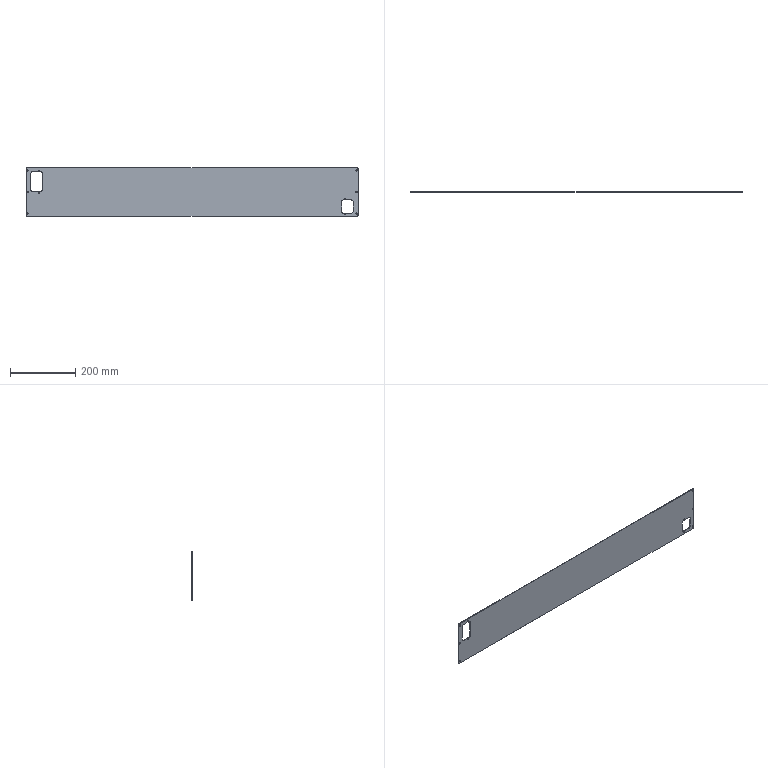Part | SolidWorks | features HoleWzd 4, Fillet 3, ICE 2, Extrusion 1, MirrorPattern 1, MoveFace 1 | 1 solid | 46 faces | box 1017 x 2 x 148 mm | volume 293852 mm3 | cylinder 32 | plane 14 | commonest cylinder face diameters 4.5 x12 3.3 x8 10 x8 4 x4
STEP:
#1=CARTESIAN_POINT('',(-504.5,0.,-2.25));
#2=VERTEX_POINT('',#1);
#3=CARTESIAN_POINT('',(-504.5,0.,2.25));
#4=VERTEX_POINT('',#3);
#5=CARTESIAN_POINT('',(-504.5,0.,0.));
#6=DIRECTION('',(0.,1.,0.));
#7=DIRECTION('',(0.,0.,1.));
#8=AXIS2_PLACEMENT_3D('',#5,#6,#7);
#9=CIRCLE('',#8,2.25);
#10=EDGE_CURVE('',#2,#4,#9,.T.);
#11=ORIENTED_EDGE('',*,*,#10,.F.);
#12=CARTESIAN_POINT('',(-504.5,2.,-2.25));
#13=VERTEX_POINT('',#12);
#14=CARTESIAN_POINT('',(-504.5,2.,-2.25));
#15=DIRECTION('',(0.,1.,0.));
#16=VECTOR('',#15,1000.);
#17=LINE('',#14,#16);
#18=EDGE_CURVE('',#2,#13,#17,.T.);
#19=ORIENTED_EDGE('',*,*,#18,.T.);
#20=CARTESIAN_POINT('',(-504.5,2.,2.25));
#21=VERTEX_POINT('',#20);
#22=CARTESIAN_POINT('',(-504.5,2.,0.));
#23=DIRECTION('',(0.,1.,0.));
#24=DIRECTION('',(0.,0.,1.));
#25=AXIS2_PLACEMENT_3D('',#22,#23,#24);
#26=CIRCLE('',#25,2.25);
#27=EDGE_CURVE('',#13,#21,#26,.T.);
#28=ORIENTED_EDGE('',*,*,#27,.T.);
#29=CARTESIAN_POINT('',(-504.5,2.,2.25));
#30=DIRECTION('',(0.,1.,0.));
#31=VECTOR('',#30,1000.);
#32=LINE('',#29,#31);
#33=EDGE_CURVE('',#4,#21,#32,.T.);
#34=ORIENTED_EDGE('',*,*,#33,.F.);
#35=EDGE_LOOP('',(#11,#19,#28,#34));
#36=FACE_OUTER_BOUND('',#35,.T.);
#37=CARTESIAN_POINT('',(-504.5,2.,0.));
#38=DIRECTION('',(0.,1.,0.));
#39=DIRECTION('',(0.,0.,1.));
#40=AXIS2_PLACEMENT_3D('',#37,#38,#39);
#41=CYLINDRICAL_SURFACE('',#40,2.25);
#42=ADVANCED_FACE('',(#36),#41,.F.);
#43=CARTESIAN_POINT('',(-504.5,0.,64.25));
#44=VERTEX_POINT('',#43);
#45=CARTESIAN_POINT('',(-504.5,0.,68.75));
#46=VERTEX_POINT('',#45);
#47=CARTESIAN_POINT('',(-504.5,0.,66.5));
#48=DIRECTION('',(0.,1.,0.));
#49=DIRECTION('',(0.,0.,1.));
#50=AXIS2_PLACEMENT_3D('',#47,#48,#49);
#51=CIRCLE('',#50,2.25);
#52=EDGE_CURVE('',#44,#46,#51,.T.);
#53=ORIENTED_EDGE('',*,*,#52,.F.);
#54=CARTESIAN_POINT('',(-504.5,2.,64.25));
#55=VERTEX_POINT('',#54);
#56=CARTESIAN_POINT('',(-504.5,2.,64.25));
#57=DIRECTION('',(0.,1.,0.));
#58=VECTOR('',#57,1000.);
#59=LINE('',#56,#58);
#60=EDGE_CURVE('',#44,#55,#59,.T.);
#61=ORIENTED_EDGE('',*,*,#60,.T.);
#62=CARTESIAN_POINT('',(-504.5,2.,68.75));
#63=VERTEX_POINT('',#62);
#64=CARTESIAN_POINT('',(-504.5,2.,66.5));
#65=DIRECTION('',(0.,1.,0.));
#66=DIRECTION('',(0.,0.,1.));
#67=AXIS2_PLACEMENT_3D('',#64,#65,#66);
#68=CIRCLE('',#67,2.25);
#69=EDGE_CURVE('',#55,#63,#68,.T.);
#70=ORIENTED_EDGE('',*,*,#69,.T.);
#71=CARTESIAN_POINT('',(-504.5,2.,68.75));
#72=DIRECTION('',(0.,1.,0.));
#73=VECTOR('',#72,1000.);
#74=LINE('',#71,#73);
#75=EDGE_CURVE('',#46,#63,#74,.T.);
#76=ORIENTED_EDGE('',*,*,#75,.F.);
#77=EDGE_LOOP('',(#53,#61,#70,#76));
#78=FACE_OUTER_BOUND('',#77,.T.);
#79=CARTESIAN_POINT('',(-504.5,2.,66.5));
#80=DIRECTION('',(0.,1.,0.));
#81=DIRECTION('',(0.,0.,1.));
#82=AXIS2_PLACEMENT_3D('',#79,#80,#81);
#83=CYLINDRICAL_SURFACE('',#82,2.25);
#84=ADVANCED_FACE('',(#78),#83,.F.);
#85=CARTESIAN_POINT('',(-504.5,0.,-68.75));
#86=VERTEX_POINT('',#85);
#87=CARTESIAN_POINT('',(-504.5,0.,-64.25));
#88=VERTEX_POINT('',#87);
#89=CARTESIAN_POINT('',(-504.5,0.,-66.5));
#90=DIRECTION('',(0.,1.,0.));
#91=DIRECTION('',(0.,0.,1.));
#92=AXIS2_PLACEMENT_3D('',#89,#90,#91);
#93=CIRCLE('',#92,2.25);
#94=EDGE_CURVE('',#86,#88,#93,.T.);
#95=ORIENTED_EDGE('',*,*,#94,.F.);
#96=CARTESIAN_POINT('',(-504.5,2.,-68.75));
#97=VERTEX_POINT('',#96);
#98=CARTESIAN_POINT('',(-504.5,2.,-68.75));
#99=DIRECTION('',(0.,1.,0.));
#100=VECTOR('',#99,1000.);
#101=LINE('',#98,#100);
#102=EDGE_CURVE('',#86,#97,#101,.T.);
#103=ORIENTED_EDGE('',*,*,#102,.T.);
#104=CARTESIAN_POINT('',(-504.5,2.,-64.25));
#105=VERTEX_POINT('',#104);
#106=CARTESIAN_POINT('',(-504.5,2.,-66.5));
#107=DIRECTION('',(0.,1.,0.));
#108=DIRECTION('',(0.,0.,1.));
#109=AXIS2_PLACEMENT_3D('',#106,#107,#108);
#110=CIRCLE('',#109,2.25);
#111=EDGE_CURVE('',#97,#105,#110,.T.);
#112=ORIENTED_EDGE('',*,*,#111,.T.);
#113=CARTESIAN_POINT('',(-504.5,2.,-64.25));
#114=DIRECTION('',(0.,1.,0.));
#115=VECTOR('',#114,1000.);
#116=LINE('',#113,#115);
#117=EDGE_CURVE('',#88,#105,#116,.T.);
#118=ORIENTED_EDGE('',*,*,#117,.F.);
#119=EDGE_LOOP('',(#95,#103,#112,#118));
#120=FACE_OUTER_BOUND('',#119,.T.);
#121=CARTESIAN_POINT('',(-504.5,2.,-66.5));
#122=DIRECTION('',(0.,1.,0.));
#123=DIRECTION('',(0.,0.,1.));
#124=AXIS2_PLACEMENT_3D('',#121,#122,#123);
#125=CYLINDRICAL_SURFACE('',#124,2.25);
#126=ADVANCED_FACE('',(#120),#125,.F.);
#127=CARTESIAN_POINT('',(468.5,0.,-69.65));
#128=VERTEX_POINT('',#127);
#129=CARTESIAN_POINT('',(468.5,0.,-66.35));
#130=VERTEX_POINT('',#129);
#131=CARTESIAN_POINT('',(468.5,0.,-68.));
#132=DIRECTION('',(0.,1.,0.));
#133=DIRECTION('',(0.,0.,1.));
#134=AXIS2_PLACEMENT_3D('',#131,#132,#133);
#135=CIRCLE('',#134,1.65);
#136=EDGE_CURVE('',#128,#130,#135,.T.);
#137=ORIENTED_EDGE('',*,*,#136,.F.);
#138=CARTESIAN_POINT('',(468.5,2.,-69.65));
#139=VERTEX_POINT('',#138);
#140=CARTESIAN_POINT('',(468.5,2.,-69.65));
#141=DIRECTION('',(0.,1.,0.));
#142=VECTOR('',#141,1000.);
#143=LINE('',#140,#142);
#144=EDGE_CURVE('',#128,#139,#143,.T.);
#145=ORIENTED_EDGE('',*,*,#144,.T.);
#146=CARTESIAN_POINT('',(468.5,2.,-66.35));
#147=VERTEX_POINT('',#146);
#148=CARTESIAN_POINT('',(468.5,2.,-68.));
#149=DIRECTION('',(0.,1.,0.));
#150=DIRECTION('',(0.,0.,1.));
#151=AXIS2_PLACEMENT_3D('',#148,#149,#150);
#152=CIRCLE('',#151,1.65);
#153=EDGE_CURVE('',#139,#147,#152,.T.);
#154=ORIENTED_EDGE('',*,*,#153,.T.);
#155=CARTESIAN_POINT('',(468.5,2.,-66.35));
#156=DIRECTION('',(0.,1.,0.));
#157=VECTOR('',#156,1000.);
#158=LINE('',#155,#157);
#159=EDGE_CURVE('',#130,#147,#158,.T.);
#160=ORIENTED_EDGE('',*,*,#159,.F.);
#161=EDGE_LOOP('',(#137,#145,#154,#160));
#162=FACE_OUTER_BOUND('',#161,.T.);
#163=CARTESIAN_POINT('',(468.5,2.,-68.));
#164=DIRECTION('',(0.,1.,0.));
#165=DIRECTION('',(0.,0.,1.));
#166=AXIS2_PLACEMENT_3D('',#163,#164,#165);
#167=CYLINDRICAL_SURFACE('',#166,1.65);
#168=ADVANCED_FACE('',(#162),#167,.F.);
#169=CARTESIAN_POINT('',(468.5,0.,-22.65));
#170=VERTEX_POINT('',#169);
#171=CARTESIAN_POINT('',(468.5,0.,-19.35));
#172=VERTEX_POINT('',#171);
#173=CARTESIAN_POINT('',(468.5,0.,-21.));
#174=DIRECTION('',(0.,1.,0.));
#175=DIRECTION('',(0.,0.,1.));
#176=AXIS2_PLACEMENT_3D('',#173,#174,#175);
#177=CIRCLE('',#176,1.65);
#178=EDGE_CURVE('',#170,#172,#177,.T.);
#179=ORIENTED_EDGE('',*,*,#178,.F.);
#180=CARTESIAN_POINT('',(468.5,2.,-22.65));
#181=VERTEX_POINT('',#180);
#182=CARTESIAN_POINT('',(468.5,2.,-22.65));
#183=DIRECTION('',(0.,1.,0.));
#184=VECTOR('',#183,1000.);
#185=LINE('',#182,#184);
#186=EDGE_CURVE('',#170,#181,#185,.T.);
#187=ORIENTED_EDGE('',*,*,#186,.T.);
#188=CARTESIAN_POINT('',(468.5,2.,-19.35));
#189=VERTEX_POINT('',#188);
#190=CARTESIAN_POINT('',(468.5,2.,-21.));
#191=DIRECTION('',(0.,1.,0.));
#192=DIRECTION('',(0.,0.,1.));
#193=AXIS2_PLACEMENT_3D('',#190,#191,#192);
#194=CIRCLE('',#193,1.65);
#195=EDGE_CURVE('',#181,#189,#194,.T.);
#196=ORIENTED_EDGE('',*,*,#195,.T.);
#197=CARTESIAN_POINT('',(468.5,2.,-19.35));
#198=DIRECTION('',(0.,1.,0.));
#199=VECTOR('',#198,1000.);
#200=LINE('',#197,#199);
#201=EDGE_CURVE('',#172,#189,#200,.T.);
#202=ORIENTED_EDGE('',*,*,#201,.F.);
#203=EDGE_LOOP('',(#179,#187,#196,#202));
#204=FACE_OUTER_BOUND('',#203,.T.);
#205=CARTESIAN_POINT('',(468.5,2.,-21.));
#206=DIRECTION('',(0.,1.,0.));
#207=DIRECTION('',(0.,0.,1.));
#208=AXIS2_PLACEMENT_3D('',#205,#206,#207);
#209=CYLINDRICAL_SURFACE('',#208,1.65);
#210=ADVANCED_FACE('',(#204),#209,.F.);
#211=CARTESIAN_POINT('',(-468.5,0.,-3.15));
#212=VERTEX_POINT('',#211);
#213=CARTESIAN_POINT('',(-468.5,0.,0.15));
#214=VERTEX_POINT('',#213);
#215=CARTESIAN_POINT('',(-468.5,0.,-1.5));
#216=DIRECTION('',(0.,1.,0.));
#217=DIRECTION('',(0.,0.,1.));
#218=AXIS2_PLACEMENT_3D('',#215,#216,#217);
#219=CIRCLE('',#218,1.65);
#220=EDGE_CURVE('',#212,#214,#219,.T.);
#221=ORIENTED_EDGE('',*,*,#220,.F.);
#222=CARTESIAN_POINT('',(-468.5,2.,-3.15));
#223=VERTEX_POINT('',#222);
#224=CARTESIAN_POINT('',(-468.5,2.,-3.15));
#225=DIRECTION('',(0.,1.,0.));
#226=VECTOR('',#225,1000.);
#227=LINE('',#224,#226);
#228=EDGE_CURVE('',#212,#223,#227,.T.);
#229=ORIENTED_EDGE('',*,*,#228,.T.);
#230=CARTESIAN_POINT('',(-468.5,2.,0.15));
#231=VERTEX_POINT('',#230);
#232=CARTESIAN_POINT('',(-468.5,2.,-1.5));
#233=DIRECTION('',(0.,1.,0.));
#234=DIRECTION('',(0.,0.,1.));
#235=AXIS2_PLACEMENT_3D('',#232,#233,#234);
#236=CIRCLE('',#235,1.65);
#237=EDGE_CURVE('',#223,#231,#236,.T.);
#238=ORIENTED_EDGE('',*,*,#237,.T.);
#239=CARTESIAN_POINT('',(-468.5,2.,0.15));
#240=DIRECTION('',(0.,1.,0.));
#241=VECTOR('',#240,1000.);
#242=LINE('',#239,#241);
#243=EDGE_CURVE('',#214,#231,#242,.T.);
#244=ORIENTED_EDGE('',*,*,#243,.F.);
#245=EDGE_LOOP('',(#221,#229,#238,#244));
#246=FACE_OUTER_BOUND('',#245,.T.);
#247=CARTESIAN_POINT('',(-468.5,2.,-1.5));
#248=DIRECTION('',(0.,1.,0.));
#249=DIRECTION('',(0.,0.,1.));
#250=AXIS2_PLACEMENT_3D('',#247,#248,#249);
#251=CYLINDRICAL_SURFACE('',#250,1.65);
#252=ADVANCED_FACE('',(#246),#251,.F.);
#253=CARTESIAN_POINT('',(-468.5,0.,63.85));
#254=VERTEX_POINT('',#253);
#255=CARTESIAN_POINT('',(-468.5,0.,67.15));
#256=VERTEX_POINT('',#255);
#257=CARTESIAN_POINT('',(-468.5,0.,65.5));
#258=DIRECTION('',(0.,1.,0.));
#259=DIRECTION('',(0.,0.,1.));
#260=AXIS2_PLACEMENT_3D('',#257,#258,#259);
#261=CIRCLE('',#260,1.65);
#262=EDGE_CURVE('',#254,#256,#261,.T.);
#263=ORIENTED_EDGE('',*,*,#262,.F.);
#264=CARTESIAN_POINT('',(-468.5,2.,63.85));
#265=VERTEX_POINT('',#264);
#266=CARTESIAN_POINT('',(-468.5,2.,63.85));
#267=DIRECTION('',(0.,1.,0.));
#268=VECTOR('',#267,1000.);
#269=LINE('',#266,#268);
#270=EDGE_CURVE('',#254,#265,#269,.T.);
#271=ORIENTED_EDGE('',*,*,#270,.T.);
#272=CARTESIAN_POINT('',(-468.5,2.,67.15));
#273=VERTEX_POINT('',#272);
#274=CARTESIAN_POINT('',(-468.5,2.,65.5));
#275=DIRECTION('',(0.,1.,0.));
#276=DIRECTION('',(0.,0.,1.));
#277=AXIS2_PLACEMENT_3D('',#274,#275,#276);
#278=CIRCLE('',#277,1.65);
#279=EDGE_CURVE('',#265,#273,#278,.T.);
#280=ORIENTED_EDGE('',*,*,#279,.T.);
#281=CARTESIAN_POINT('',(-468.5,2.,67.15));
#282=DIRECTION('',(0.,1.,0.));
#283=VECTOR('',#282,1000.);
#284=LINE('',#281,#283);
#285=EDGE_CURVE('',#256,#273,#284,.T.);
#286=ORIENTED_EDGE('',*,*,#285,.F.);
#287=EDGE_LOOP('',(#263,#271,#280,#286));
#288=FACE_OUTER_BOUND('',#287,.T.);
#289=CARTESIAN_POINT('',(-468.5,2.,65.5));
#290=DIRECTION('',(0.,1.,0.));
#291=DIRECTION('',(0.,0.,1.));
#292=AXIS2_PLACEMENT_3D('',#289,#290,#291);
#293=CYLINDRICAL_SURFACE('',#292,1.65);
#294=ADVANCED_FACE('',(#288),#293,.F.);
#295=CARTESIAN_POINT('',(504.5,0.,-2.25));
#296=VERTEX_POINT('',#295);
#297=CARTESIAN_POINT('',(504.5,0.,2.25));
#298=VERTEX_POINT('',#297);
#299=CARTESIAN_POINT('',(504.5,0.,0.));
#300=DIRECTION('',(0.,1.,0.));
#301=DIRECTION('',(0.,0.,1.));
#302=AXIS2_PLACEMENT_3D('',#299,#300,#301);
#303=CIRCLE('',#302,2.25);
#304=EDGE_CURVE('',#296,#298,#303,.T.);
#305=ORIENTED_EDGE('',*,*,#304,.F.);
#306=CARTESIAN_POINT('',(504.5,2.,-2.25));
#307=VERTEX_POINT('',#306);
#308=CARTESIAN_POINT('',(504.5,2.,-2.25));
#309=DIRECTION('',(0.,1.,0.));
#310=VECTOR('',#309,1000.);
#311=LINE('',#308,#310);
#312=EDGE_CURVE('',#296,#307,#311,.T.);
#313=ORIENTED_EDGE('',*,*,#312,.T.);
#314=CARTESIAN_POINT('',(504.5,2.,2.25));
#315=VERTEX_POINT('',#314);
#316=CARTESIAN_POINT('',(504.5,2.,0.));
#317=DIRECTION('',(0.,1.,0.));
#318=DIRECTION('',(0.,0.,1.));
#319=AXIS2_PLACEMENT_3D('',#316,#317,#318);
#320=CIRCLE('',#319,2.25);
#321=EDGE_CURVE('',#307,#315,#320,.T.);
#322=ORIENTED_EDGE('',*,*,#321,.T.);
#323=CARTESIAN_POINT('',(504.5,2.,2.25));
#324=DIRECTION('',(0.,1.,0.));
#325=VECTOR('',#324,1000.);
#326=LINE('',#323,#325);
#327=EDGE_CURVE('',#298,#315,#326,.T.);
#328=ORIENTED_EDGE('',*,*,#327,.F.);
#329=EDGE_LOOP('',(#305,#313,#322,#328));
#330=FACE_OUTER_BOUND('',#329,.T.);
#331=CARTESIAN_POINT('',(504.5,2.,0.));
#332=DIRECTION('',(0.,1.,0.));
#333=DIRECTION('',(0.,0.,1.));
#334=AXIS2_PLACEMENT_3D('',#331,#332,#333);
#335=CYLINDRICAL_SURFACE('',#334,2.25);
#336=ADVANCED_FACE('',(#330),#335,.F.);
#337=CARTESIAN_POINT('',(504.5,0.,64.25));
#338=VERTEX_POINT('',#337);
#339=CARTESIAN_POINT('',(504.5,0.,68.75));
#340=VERTEX_POINT('',#339);
#341=CARTESIAN_POINT('',(504.5,0.,66.5));
#342=DIRECTION('',(0.,1.,0.));
#343=DIRECTION('',(0.,0.,1.));
#344=AXIS2_PLACEMENT_3D('',#341,#342,#343);
#345=CIRCLE('',#344,2.25);
#346=EDGE_CURVE('',#338,#340,#345,.T.);
#347=ORIENTED_EDGE('',*,*,#346,.F.);
#348=CARTESIAN_POINT('',(504.5,2.,64.25));
#349=VERTEX_POINT('',#348);
#350=CARTESIAN_POINT('',(504.5,2.,64.25));
#351=DIRECTION('',(0.,1.,0.));
#352=VECTOR('',#351,1000.);
#353=LINE('',#350,#352);
#354=EDGE_CURVE('',#338,#349,#353,.T.);
#355=ORIENTED_EDGE('',*,*,#354,.T.);
#356=CARTESIAN_POINT('',(504.5,2.,68.75));
#357=VERTEX_POINT('',#356);
#358=CARTESIAN_POINT('',(504.5,2.,66.5));
#359=DIRECTION('',(0.,1.,0.));
#360=DIRECTION('',(0.,0.,1.));
#361=AXIS2_PLACEMENT_3D('',#358,#359,#360);
#362=CIRCLE('',#361,2.25);
#363=EDGE_CURVE('',#349,#357,#362,.T.);
#364=ORIENTED_EDGE('',*,*,#363,.T.);
#365=CARTESIAN_POINT('',(504.5,2.,68.75));
#366=DIRECTION('',(0.,1.,0.));
#367=VECTOR('',#366,1000.);
#368=LINE('',#365,#367);
#369=EDGE_CURVE('',#340,#357,#368,.T.);
#370=ORIENTED_EDGE('',*,*,#369,.F.);
#371=EDGE_LOOP('',(#347,#355,#364,#370));
#372=FACE_OUTER_BOUND('',#371,.T.);
#373=CARTESIAN_POINT('',(504.5,2.,66.5));
#374=DIRECTION('',(0.,1.,0.));
#375=DIRECTION('',(0.,0.,1.));
#376=AXIS2_PLACEMENT_3D('',#373,#374,#375);
#377=CYLINDRICAL_SURFACE('',#376,2.25);
#378=ADVANCED_FACE('',(#372),#377,.F.);
#379=CARTESIAN_POINT('',(504.5,0.,-68.75));
#380=VERTEX_POINT('',#379);
#381=CARTESIAN_POINT('',(504.5,0.,-64.25));
#382=VERTEX_POINT('',#381);
#383=CARTESIAN_POINT('',(504.5,0.,-66.5));
#384=DIRECTION('',(0.,1.,0.));
#385=DIRECTION('',(0.,0.,1.));
#386=AXIS2_PLACEMENT_3D('',#383,#384,#385);
#387=CIRCLE('',#386,2.25);
#388=EDGE_CURVE('',#380,#382,#387,.T.);
#389=ORIENTED_EDGE('',*,*,#388,.F.);
#390=CARTESIAN_POINT('',(504.5,2.,-68.75));
#391=VERTEX_POINT('',#390);
#392=CARTESIAN_POINT('',(504.5,2.,-68.75));
#393=DIRECTION('',(0.,1.,0.));
#394=VECTOR('',#393,1000.);
#395=LINE('',#392,#394);
#396=EDGE_CURVE('',#380,#391,#395,.T.);
#397=ORIENTED_EDGE('',*,*,#396,.T.);
#398=CARTESIAN_POINT('',(504.5,2.,-64.25));
#399=VERTEX_POINT('',#398);
#400=CARTESIAN_POINT('',(504.5,2.,-66.5));
#401=DIRECTION('',(0.,1.,0.));
#402=DIRECTION('',(0.,0.,1.));
#403=AXIS2_PLACEMENT_3D('',#400,#401,#402);
#404=CIRCLE('',#403,2.25);
#405=EDGE_CURVE('',#391,#399,#404,.T.);
#406=ORIENTED_EDGE('',*,*,#405,.T.);
#407=CARTESIAN_POINT('',(504.5,2.,-64.25));
#408=DIRECTION('',(0.,1.,0.));
#409=VECTOR('',#408,1000.);
#410=LINE('',#407,#409);
#411=EDGE_CURVE('',#382,#399,#410,.T.);
#412=ORIENTED_EDGE('',*,*,#411,.F.);
#413=EDGE_LOOP('',(#389,#397,#406,#412));
#414=FACE_OUTER_BOUND('',#413,.T.);
#415=CARTESIAN_POINT('',(504.5,2.,-66.5));
#416=DIRECTION('',(0.,1.,0.));
#417=DIRECTION('',(0.,0.,1.));
#418=AXIS2_PLACEMENT_3D('',#415,#416,#417);
#419=CYLINDRICAL_SURFACE('',#418,2.25);
#420=ADVANCED_FACE('',(#414),#419,.F.);
#421=CARTESIAN_POINT('',(508.5,0.,72.));
#422=VERTEX_POINT('',#421);
#423=CARTESIAN_POINT('',(508.5,0.,-72.));
#424=VERTEX_POINT('',#423);
#425=CARTESIAN_POINT('',(508.5,0.,-74.));
#426=DIRECTION('',(0.,0.,-1.));
#427=VECTOR('',#426,1000.);
#428=LINE('',#425,#427);
#429=EDGE_CURVE('',#422,#424,#428,.T.);
#430=ORIENTED_EDGE('',*,*,#429,.T.);
#431=CARTESIAN_POINT('',(508.5,2.,-72.));
#432=VERTEX_POINT('',#431);
#433=CARTESIAN_POINT('',(508.5,2.,-72.));
#434=DIRECTION('',(0.,1.,0.));
#435=VECTOR('',#434,1000.);
#436=LINE('',#433,#435);
#437=EDGE_CURVE('',#424,#432,#436,.T.);
#438=ORIENTED_EDGE('',*,*,#437,.T.);
#439=CARTESIAN_POINT('',(508.5,2.,72.));
#440=VERTEX_POINT('',#439);
#441=CARTESIAN_POINT('',(508.5,2.,-74.));
#442=DIRECTION('',(0.,0.,-1.));
#443=VECTOR('',#442,1000.);
#444=LINE('',#441,#443);
#445=EDGE_CURVE('',#440,#432,#444,.T.);
#446=ORIENTED_EDGE('',*,*,#445,.F.);
#447=CARTESIAN_POINT('',(508.5,2.,72.));
#448=DIRECTION('',(0.,-1.,0.));
#449=VECTOR('',#448,1000.);
#450=LINE('',#447,#449);
#451=EDGE_CURVE('',#440,#422,#450,.T.);
#452=ORIENTED_EDGE('',*,*,#451,.T.);
#453=EDGE_LOOP('',(#430,#438,#446,#452));
#454=FACE_OUTER_BOUND('',#453,.T.);
#455=CARTESIAN_POINT('',(508.5,2.,-74.));
#456=DIRECTION('',(-1.,0.,0.));
#457=DIRECTION('',(0.,0.,1.));
#458=AXIS2_PLACEMENT_3D('',#455,#456,#457);
#459=PLANE('',#458);
#460=ADVANCED_FACE('',(#454),#459,.F.);
#461=CARTESIAN_POINT('',(506.5,0.,-74.));
#462=VERTEX_POINT('',#461);
#463=CARTESIAN_POINT('',(-506.5,0.,-74.));
#464=VERTEX_POINT('',#463);
#465=CARTESIAN_POINT('',(-508.5,0.,-74.));
#466=DIRECTION('',(-1.,0.,0.));
#467=VECTOR('',#466,1000.);
#468=LINE('',#465,#467);
#469=EDGE_CURVE('',#462,#464,#468,.T.);
#470=ORIENTED_EDGE('',*,*,#469,.T.);
#471=CARTESIAN_POINT('',(-506.5,2.,-74.));
#472=VERTEX_POINT('',#471);
#473=CARTESIAN_POINT('',(-506.5,2.,-74.));
#474=DIRECTION('',(0.,1.,0.));
#475=VECTOR('',#474,1000.);
#476=LINE('',#473,#475);
#477=EDGE_CURVE('',#464,#472,#476,.T.);
#478=ORIENTED_EDGE('',*,*,#477,.T.);
#479=CARTESIAN_POINT('',(506.5,2.,-74.));
#480=VERTEX_POINT('',#479);
#481=CARTESIAN_POINT('',(-508.5,2.,-74.));
#482=DIRECTION('',(-1.,0.,0.));
#483=VECTOR('',#482,1000.);
#484=LINE('',#481,#483);
#485=EDGE_CURVE('',#480,#472,#484,.T.);
#486=ORIENTED_EDGE('',*,*,#485,.F.);
#487=CARTESIAN_POINT('',(506.5,2.,-74.));
#488=DIRECTION('',(0.,-1.,0.));
#489=VECTOR('',#488,1000.);
#490=LINE('',#487,#489);
#491=EDGE_CURVE('',#480,#462,#490,.T.);
#492=ORIENTED_EDGE('',*,*,#491,.T.);
#493=EDGE_LOOP('',(#470,#478,#486,#492));
#494=FACE_OUTER_BOUND('',#493,.T.);
#495=CARTESIAN_POINT('',(-508.5,2.,-74.));
#496=DIRECTION('',(0.,0.,1.));
#497=DIRECTION('',(1.,0.,0.));
#498=AXIS2_PLACEMENT_3D('',#495,#496,#497);
#499=PLANE('',#498);
#500=ADVANCED_FACE('',(#494),#499,.F.);
#501=CARTESIAN_POINT('',(-508.5,2.,-72.));
#502=VERTEX_POINT('',#501);
#503=CARTESIAN_POINT('',(-508.5,2.,72.));
#504=VERTEX_POINT('',#503);
#505=CARTESIAN_POINT('',(-508.5,2.,-74.));
#506=DIRECTION('',(0.,0.,1.));
#507=VECTOR('',#506,1000.);
#508=LINE('',#505,#507);
#509=EDGE_CURVE('',#502,#504,#508,.T.);
#510=ORIENTED_EDGE('',*,*,#509,.F.);
#511=CARTESIAN_POINT('',(-508.5,0.,-72.));
#512=VERTEX_POINT('',#511);
#513=CARTESIAN_POINT('',(-508.5,2.,-72.));
#514=DIRECTION('',(0.,-1.,0.));
#515=VECTOR('',#514,1000.);
#516=LINE('',#513,#515);
#517=EDGE_CURVE('',#502,#512,#516,.T.);
#518=ORIENTED_EDGE('',*,*,#517,.T.);
#519=CARTESIAN_POINT('',(-508.5,0.,72.));
#520=VERTEX_POINT('',#519);
#521=CARTESIAN_POINT('',(-508.5,0.,-74.));
#522=DIRECTION('',(0.,0.,1.));
#523=VECTOR('',#522,1000.);
#524=LINE('',#521,#523);
#525=EDGE_CURVE('',#512,#520,#524,.T.);
#526=ORIENTED_EDGE('',*,*,#525,.T.);
#527=CARTESIAN_POINT('',(-508.5,2.,72.));
#528=DIRECTION('',(0.,1.,0.));
#529=VECTOR('',#528,1000.);
#530=LINE('',#527,#529);
#531=EDGE_CURVE('',#520,#504,#530,.T.);
#532=ORIENTED_EDGE('',*,*,#531,.T.);
#533=EDGE_LOOP('',(#510,#518,#526,#532));
#534=FACE_OUTER_BOUND('',#533,.T.);
#535=CARTESIAN_POINT('',(-508.5,2.,-74.));
#536=DIRECTION('',(1.,0.,0.));
#537=DIRECTION('',(0.,0.,-1.));
#538=AXIS2_PLACEMENT_3D('',#535,#536,#537);
#539=PLANE('',#538);
#540=ADVANCED_FACE('',(#534),#539,.F.);
#541=CARTESIAN_POINT('',(-506.5,2.,74.));
#542=VERTEX_POINT('',#541);
#543=CARTESIAN_POINT('',(506.5,2.,74.));
#544=VERTEX_POINT('',#543);
#545=CARTESIAN_POINT('',(-508.5,2.,74.));
#546=DIRECTION('',(1.,0.,0.));
#547=VECTOR('',#546,1000.);
#548=LINE('',#545,#547);
#549=EDGE_CURVE('',#542,#544,#548,.T.);
#550=ORIENTED_EDGE('',*,*,#549,.F.);
#551=CARTESIAN_POINT('',(-506.5,0.,74.));
#552=VERTEX_POINT('',#551);
#553=CARTESIAN_POINT('',(-506.5,2.,74.));
#554=DIRECTION('',(0.,-1.,0.));
#555=VECTOR('',#554,1000.);
#556=LINE('',#553,#555);
#557=EDGE_CURVE('',#542,#552,#556,.T.);
#558=ORIENTED_EDGE('',*,*,#557,.T.);
#559=CARTESIAN_POINT('',(506.5,0.,74.));
#560=VERTEX_POINT('',#559);
#561=CARTESIAN_POINT('',(-508.5,0.,74.));
#562=DIRECTION('',(1.,0.,0.));
#563=VECTOR('',#562,1000.);
#564=LINE('',#561,#563);
#565=EDGE_CURVE('',#552,#560,#564,.T.);
#566=ORIENTED_EDGE('',*,*,#565,.T.);
#567=CARTESIAN_POINT('',(506.5,2.,74.));
#568=DIRECTION('',(0.,1.,0.));
#569=VECTOR('',#568,1000.);
#570=LINE('',#567,#569);
#571=EDGE_CURVE('',#560,#544,#570,.T.);
#572=ORIENTED_EDGE('',*,*,#571,.T.);
#573=EDGE_LOOP('',(#550,#558,#566,#572));
#574=FACE_OUTER_BOUND('',#573,.T.);
#575=CARTESIAN_POINT('',(-508.5,2.,74.));
#576=DIRECTION('',(0.,0.,-1.));
#577=DIRECTION('',(-1.,0.,0.));
#578=AXIS2_PLACEMENT_3D('',#575,#576,#577);
#579=PLANE('',#578);
#580=ADVANCED_FACE('',(#574),#579,.F.);
#581=CARTESIAN_POINT('',(-504.5,2.,0.));
#582=DIRECTION('',(0.,1.,0.));
#583=DIRECTION('',(0.,0.,1.));
#584=AXIS2_PLACEMENT_3D('',#581,#582,#583);
#585=CIRCLE('',#584,2.25);
#586=EDGE_CURVE('',#21,#13,#585,.T.);
#587=ORIENTED_EDGE('',*,*,#586,.F.);
#588=ORIENTED_EDGE('',*,*,#27,.F.);
#589=EDGE_LOOP('',(#587,#588));
#590=FACE_BOUND('',#589,.T.);
#591=CARTESIAN_POINT('',(-504.5,2.,66.5));
#592=DIRECTION('',(0.,1.,0.));
#593=DIRECTION('',(0.,0.,1.));
#594=AXIS2_PLACEMENT_3D('',#591,#592,#593);
#595=CIRCLE('',#594,2.25);
#596=EDGE_CURVE('',#63,#55,#595,.T.);
#597=ORIENTED_EDGE('',*,*,#596,.F.);
#598=ORIENTED_EDGE('',*,*,#69,.F.);
#599=EDGE_LOOP('',(#597,#598));
#600=FACE_BOUND('',#599,.T.);
#601=CARTESIAN_POINT('',(-504.5,2.,-66.5));
#602=DIRECTION('',(0.,1.,0.));
#603=DIRECTION('',(0.,0.,1.));
#604=AXIS2_PLACEMENT_3D('',#601,#602,#603);
#605=CIRCLE('',#604,2.25);
#606=EDGE_CURVE('',#105,#97,#605,.T.);
#607=ORIENTED_EDGE('',*,*,#606,.F.);
#608=ORIENTED_EDGE('',*,*,#111,.F.);
#609=EDGE_LOOP('',(#607,#608));
#610=FACE_BOUND('',#609,.T.);
#611=CARTESIAN_POINT('',(468.5,2.,-68.));
#612=DIRECTION('',(0.,1.,0.));
#613=DIRECTION('',(0.,0.,1.));
#614=AXIS2_PLACEMENT_3D('',#611,#612,#613);
#615=CIRCLE('',#614,1.65);
#616=EDGE_CURVE('',#147,#139,#615,.T.);
#617=ORIENTED_EDGE('',*,*,#616,.F.);
#618=ORIENTED_EDGE('',*,*,#153,.F.);
#619=EDGE_LOOP('',(#617,#618));
#620=FACE_BOUND('',#619,.T.);
#621=CARTESIAN_POINT('',(468.5,2.,-21.));
#622=DIRECTION('',(0.,1.,0.));
#623=DIRECTION('',(0.,0.,1.));
#624=AXIS2_PLACEMENT_3D('',#621,#622,#623);
#625=CIRCLE('',#624,1.65);
#626=EDGE_CURVE('',#189,#181,#625,.T.);
#627=ORIENTED_EDGE('',*,*,#626,.F.);
#628=ORIENTED_EDGE('',*,*,#195,.F.);
#629=EDGE_LOOP('',(#627,#628));
#630=FACE_BOUND('',#629,.T.);
#631=CARTESIAN_POINT('',(-468.5,2.,-1.5));
#632=DIRECTION('',(0.,1.,0.));
#633=DIRECTION('',(0.,0.,1.));
#634=AXIS2_PLACEMENT_3D('',#631,#632,#633);
#635=CIRCLE('',#634,1.65);
#636=EDGE_CURVE('',#231,#223,#635,.T.);
#637=ORIENTED_EDGE('',*,*,#636,.F.);
#638=ORIENTED_EDGE('',*,*,#237,.F.);
#639=EDGE_LOOP('',(#637,#638));
#640=FACE_BOUND('',#639,.T.);
#641=CARTESIAN_POINT('',(-468.5,2.,65.5));
#642=DIRECTION('',(0.,1.,0.));
#643=DIRECTION('',(0.,0.,1.));
#644=AXIS2_PLACEMENT_3D('',#641,#642,#643);
#645=CIRCLE('',#644,1.65);
#646=EDGE_CURVE('',#273,#265,#645,.T.);
#647=ORIENTED_EDGE('',*,*,#646,.F.);
#648=ORIENTED_EDGE('',*,*,#279,.F.);
#649=EDGE_LOOP('',(#647,#648));
#650=FACE_BOUND('',#649,.T.);
#651=CARTESIAN_POINT('',(-493.5,2.,7.));
#652=VERTEX_POINT('',#651);
#653=CARTESIAN_POINT('',(-493.5,2.,57.));
#654=VERTEX_POINT('',#653);
#655=CARTESIAN_POINT('',(-493.5,2.,22.));
#656=DIRECTION('',(0.,0.,1.));
#657=VECTOR('',#656,1000.);
#658=LINE('',#655,#657);
#659=EDGE_CURVE('',#652,#654,#658,.T.);
#660=ORIENTED_EDGE('',*,*,#659,.F.);
#661=CARTESIAN_POINT('',(-488.5,2.,2.));
#662=VERTEX_POINT('',#661);
#663=CARTESIAN_POINT('',(-488.5,2.,7.));
#664=DIRECTION('',(0.,-1.,0.));
#665=DIRECTION('',(0.,0.,1.));
#666=AXIS2_PLACEMENT_3D('',#663,#664,#665);
#667=CIRCLE('',#666,5.);
#668=EDGE_CURVE('',#652,#662,#667,.T.);
#669=ORIENTED_EDGE('',*,*,#668,.T.);
#670=CARTESIAN_POINT('',(-463.5,2.,2.));
#671=VERTEX_POINT('',#670);
#672=CARTESIAN_POINT('',(-458.5,2.,2.));
#673=DIRECTION('',(-1.,0.,0.));
#674=VECTOR('',#673,1000.);
#675=LINE('',#672,#674);
#676=EDGE_CURVE('',#671,#662,#675,.T.);
#677=ORIENTED_EDGE('',*,*,#676,.F.);
#678=CARTESIAN_POINT('',(-458.5,2.,7.));
#679=VERTEX_POINT('',#678);
#680=CARTESIAN_POINT('',(-463.5,2.,7.));
#681=DIRECTION('',(0.,-1.,0.));
#682=DIRECTION('',(0.,0.,1.));
#683=AXIS2_PLACEMENT_3D('',#680,#681,#682);
#684=CIRCLE('',#683,5.);
#685=EDGE_CURVE('',#671,#679,#684,.T.);
#686=ORIENTED_EDGE('',*,*,#685,.T.);
#687=CARTESIAN_POINT('',(-458.5,2.,57.));
#688=VERTEX_POINT('',#687);
#689=CARTESIAN_POINT('',(-458.5,2.,22.));
#690=DIRECTION('',(0.,0.,-1.));
#691=VECTOR('',#690,1000.);
#692=LINE('',#689,#691);
#693=EDGE_CURVE('',#688,#679,#692,.T.);
#694=ORIENTED_EDGE('',*,*,#693,.F.);
#695=CARTESIAN_POINT('',(-463.5,2.,62.));
#696=VERTEX_POINT('',#695);
#697=CARTESIAN_POINT('',(-463.5,2.,57.));
#698=DIRECTION('',(0.,-1.,0.));
#699=DIRECTION('',(0.,0.,1.));
#700=AXIS2_PLACEMENT_3D('',#697,#698,#699);
#701=CIRCLE('',#700,5.);
#702=EDGE_CURVE('',#688,#696,#701,.T.);
#703=ORIENTED_EDGE('',*,*,#702,.T.);
#704=CARTESIAN_POINT('',(-488.5,2.,62.));
#705=VERTEX_POINT('',#704);
#706=CARTESIAN_POINT('',(-458.5,2.,62.));
#707=DIRECTION('',(1.,0.,0.));
#708=VECTOR('',#707,1000.);
#709=LINE('',#706,#708);
#710=EDGE_CURVE('',#705,#696,#709,.T.);
#711=ORIENTED_EDGE('',*,*,#710,.F.);
#712=CARTESIAN_POINT('',(-488.5,2.,57.));
#713=DIRECTION('',(0.,-1.,0.));
#714=DIRECTION('',(0.,0.,1.));
#715=AXIS2_PLACEMENT_3D('',#712,#713,#714);
#716=CIRCLE('',#715,5.);
#717=EDGE_CURVE('',#705,#654,#716,.T.);
#718=ORIENTED_EDGE('',*,*,#717,.T.);
#719=EDGE_LOOP('',(#660,#669,#677,#686,#694,#703,#711,#718));
#720=FACE_BOUND('',#719,.T.);
#721=CARTESIAN_POINT('',(493.5,2.,-29.5));
#722=VERTEX_POINT('',#721);
#723=CARTESIAN_POINT('',(493.5,2.,-59.5));
#724=VERTEX_POINT('',#723);
#725=CARTESIAN_POINT('',(493.5,2.,-64.5));
#726=DIRECTION('',(0.,0.,-1.));
#727=VECTOR('',#726,1000.);
#728=LINE('',#725,#727);
#729=EDGE_CURVE('',#722,#724,#728,.T.);
#730=ORIENTED_EDGE('',*,*,#729,.F.);
#731=CARTESIAN_POINT('',(488.5,2.,-24.5));
#732=VERTEX_POINT('',#731);
#733=CARTESIAN_POINT('',(488.5,2.,-29.5));
#734=DIRECTION('',(0.,-1.,0.));
#735=DIRECTION('',(0.,0.,1.));
#736=AXIS2_PLACEMENT_3D('',#733,#734,#735);
#737=CIRCLE('',#736,5.);
#738=EDGE_CURVE('',#722,#732,#737,.T.);
#739=ORIENTED_EDGE('',*,*,#738,.T.);
#740=CARTESIAN_POINT('',(463.5,2.,-24.5));
#741=VERTEX_POINT('',#740);
#742=CARTESIAN_POINT('',(458.5,2.,-24.5));
#743=DIRECTION('',(1.,0.,0.));
#744=VECTOR('',#743,1000.);
#745=LINE('',#742,#744);
#746=EDGE_CURVE('',#741,#732,#745,.T.);
#747=ORIENTED_EDGE('',*,*,#746,.F.);
#748=CARTESIAN_POINT('',(458.5,2.,-29.5));
#749=VERTEX_POINT('',#748);
#750=CARTESIAN_POINT('',(463.5,2.,-29.5));
#751=DIRECTION('',(0.,-1.,0.));
#752=DIRECTION('',(0.,0.,1.));
#753=AXIS2_PLACEMENT_3D('',#750,#751,#752);
#754=CIRCLE('',#753,5.);
#755=EDGE_CURVE('',#741,#749,#754,.T.);
#756=ORIENTED_EDGE('',*,*,#755,.T.);
#757=CARTESIAN_POINT('',(458.5,2.,-59.5));
#758=VERTEX_POINT('',#757);
#759=CARTESIAN_POINT('',(458.5,2.,-64.5));
#760=DIRECTION('',(0.,0.,1.));
#761=VECTOR('',#760,1000.);
#762=LINE('',#759,#761);
#763=EDGE_CURVE('',#758,#749,#762,.T.);
#764=ORIENTED_EDGE('',*,*,#763,.F.);
#765=CARTESIAN_POINT('',(463.5,2.,-64.5));
#766=VERTEX_POINT('',#765);
#767=CARTESIAN_POINT('',(463.5,2.,-59.5));
#768=DIRECTION('',(0.,-1.,0.));
#769=DIRECTION('',(0.,0.,1.));
#770=AXIS2_PLACEMENT_3D('',#767,#768,#769);
#771=CIRCLE('',#770,5.);
#772=EDGE_CURVE('',#758,#766,#771,.T.);
#773=ORIENTED_EDGE('',*,*,#772,.T.);
#774=CARTESIAN_POINT('',(488.5,2.,-64.5));
#775=VERTEX_POINT('',#774);
#776=CARTESIAN_POINT('',(458.5,2.,-64.5));
#777=DIRECTION('',(-1.,0.,0.));
#778=VECTOR('',#777,1000.);
#779=LINE('',#776,#778);
#780=EDGE_CURVE('',#775,#766,#779,.T.);
#781=ORIENTED_EDGE('',*,*,#780,.F.);
#782=CARTESIAN_POINT('',(488.5,2.,-59.5));
#783=DIRECTION('',(0.,-1.,0.));
#784=DIRECTION('',(0.,0.,1.));
#785=AXIS2_PLACEMENT_3D('',#782,#783,#784);
#786=CIRCLE('',#785,5.);
#787=EDGE_CURVE('',#775,#724,#786,.T.);
#788=ORIENTED_EDGE('',*,*,#787,.T.);
#789=EDGE_LOOP('',(#730,#739,#747,#756,#764,#773,#781,#788));
#790=FACE_BOUND('',#789,.T.);
#791=CARTESIAN_POINT('',(504.5,2.,0.));
#792=DIRECTION('',(0.,1.,0.));
#793=DIRECTION('',(0.,0.,1.));
#794=AXIS2_PLACEMENT_3D('',#791,#792,#793);
#795=CIRCLE('',#794,2.25);
#796=EDGE_CURVE('',#315,#307,#795,.T.);
#797=ORIENTED_EDGE('',*,*,#796,.F.);
#798=ORIENTED_EDGE('',*,*,#321,.F.);
#799=EDGE_LOOP('',(#797,#798));
#800=FACE_BOUND('',#799,.T.);
#801=CARTESIAN_POINT('',(504.5,2.,66.5));
#802=DIRECTION('',(0.,1.,0.));
#803=DIRECTION('',(0.,0.,1.));
#804=AXIS2_PLACEMENT_3D('',#801,#802,#803);
#805=CIRCLE('',#804,2.25);
#806=EDGE_CURVE('',#357,#349,#805,.T.);
#807=ORIENTED_EDGE('',*,*,#806,.F.);
#808=ORIENTED_EDGE('',*,*,#363,.F.);
#809=EDGE_LOOP('',(#807,#808));
#810=FACE_BOUND('',#809,.T.);
#811=CARTESIAN_POINT('',(504.5,2.,-66.5));
#812=DIRECTION('',(0.,1.,0.));
#813=DIRECTION('',(0.,0.,1.));
#814=AXIS2_PLACEMENT_3D('',#811,#812,#813);
#815=CIRCLE('',#814,2.25);
#816=EDGE_CURVE('',#399,#391,#815,.T.);
#817=ORIENTED_EDGE('',*,*,#816,.F.);
#818=ORIENTED_EDGE('',*,*,#405,.F.);
#819=EDGE_LOOP('',(#817,#818));
#820=FACE_BOUND('',#819,.T.);
#821=ORIENTED_EDGE('',*,*,#485,.T.);
#822=CARTESIAN_POINT('',(-506.5,2.,-72.));
#823=DIRECTION('',(0.,1.,0.));
#824=DIRECTION('',(0.,0.,1.));
#825=AXIS2_PLACEMENT_3D('',#822,#823,#824);
#826=CIRCLE('',#825,2.);
#827=EDGE_CURVE('',#472,#502,#826,.T.);
#828=ORIENTED_EDGE('',*,*,#827,.T.);
#829=ORIENTED_EDGE('',*,*,#509,.T.);
#830=CARTESIAN_POINT('',(-506.5,2.,72.));
#831=DIRECTION('',(0.,1.,0.));
#832=DIRECTION('',(0.,0.,1.));
#833=AXIS2_PLACEMENT_3D('',#830,#831,#832);
#834=CIRCLE('',#833,2.);
#835=EDGE_CURVE('',#504,#542,#834,.T.);
#836=ORIENTED_EDGE('',*,*,#835,.T.);
#837=ORIENTED_EDGE('',*,*,#549,.T.);
#838=CARTESIAN_POINT('',(506.5,2.,72.));
#839=DIRECTION('',(0.,1.,0.));
#840=DIRECTION('',(0.,0.,1.));
#841=AXIS2_PLACEMENT_3D('',#838,#839,#840);
#842=CIRCLE('',#841,2.);
#843=EDGE_CURVE('',#544,#440,#842,.T.);
#844=ORIENTED_EDGE('',*,*,#843,.T.);
#845=ORIENTED_EDGE('',*,*,#445,.T.);
#846=CARTESIAN_POINT('',(506.5,2.,-72.));
#847=DIRECTION('',(0.,1.,0.));
#848=DIRECTION('',(0.,0.,1.));
#849=AXIS2_PLACEMENT_3D('',#846,#847,#848);
#850=CIRCLE('',#849,2.);
#851=EDGE_CURVE('',#432,#480,#850,.T.);
#852=ORIENTED_EDGE('',*,*,#851,.T.);
#853=EDGE_LOOP('',(#821,#828,#829,#836,#837,#844,#845,#852));
#854=FACE_OUTER_BOUND('',#853,.T.);
#855=CARTESIAN_POINT('',(0.,2.,0.));
#856=DIRECTION('',(0.,1.,0.));
#857=DIRECTION('',(0.,0.,1.));
#858=AXIS2_PLACEMENT_3D('',#855,#856,#857);
#859=PLANE('',#858);
#860=ADVANCED_FACE('',(#590,#600,#610,#620,#630,#640,#650,#720,#790,#800,#810,#820,#854),#859,.T.);
#861=CARTESIAN_POINT('',(-504.5,0.,0.));
#862=DIRECTION('',(0.,1.,0.));
#863=DIRECTION('',(0.,0.,1.));
#864=AXIS2_PLACEMENT_3D('',#861,#862,#863);
#865=CIRCLE('',#864,2.25);
#866=EDGE_CURVE('',#4,#2,#865,.T.);
#867=ORIENTED_EDGE('',*,*,#866,.T.);
#868=ORIENTED_EDGE('',*,*,#10,.T.);
#869=EDGE_LOOP('',(#867,#868));
#870=FACE_BOUND('',#869,.T.);
#871=CARTESIAN_POINT('',(-504.5,0.,66.5));
#872=DIRECTION('',(0.,1.,0.));
#873=DIRECTION('',(0.,0.,1.));
#874=AXIS2_PLACEMENT_3D('',#871,#872,#873);
#875=CIRCLE('',#874,2.25);
#876=EDGE_CURVE('',#46,#44,#875,.T.);
#877=ORIENTED_EDGE('',*,*,#876,.T.);
#878=ORIENTED_EDGE('',*,*,#52,.T.);
#879=EDGE_LOOP('',(#877,#878));
#880=FACE_BOUND('',#879,.T.);
#881=CARTESIAN_POINT('',(-504.5,0.,-66.5));
#882=DIRECTION('',(0.,1.,0.));
#883=DIRECTION('',(0.,0.,1.));
#884=AXIS2_PLACEMENT_3D('',#881,#882,#883);
#885=CIRCLE('',#884,2.25);
#886=EDGE_CURVE('',#88,#86,#885,.T.);
#887=ORIENTED_EDGE('',*,*,#886,.T.);
#888=ORIENTED_EDGE('',*,*,#94,.T.);
#889=EDGE_LOOP('',(#887,#888));
#890=FACE_BOUND('',#889,.T.);
#891=CARTESIAN_POINT('',(468.5,0.,-68.));
#892=DIRECTION('',(0.,1.,0.));
#893=DIRECTION('',(0.,0.,1.));
#894=AXIS2_PLACEMENT_3D('',#891,#892,#893);
#895=CIRCLE('',#894,1.65);
#896=EDGE_CURVE('',#130,#128,#895,.T.);
#897=ORIENTED_EDGE('',*,*,#896,.T.);
#898=ORIENTED_EDGE('',*,*,#136,.T.);
#899=EDGE_LOOP('',(#897,#898));
#900=FACE_BOUND('',#899,.T.);
#901=CARTESIAN_POINT('',(468.5,0.,-21.));
#902=DIRECTION('',(0.,1.,0.));
#903=DIRECTION('',(0.,0.,1.));
#904=AXIS2_PLACEMENT_3D('',#901,#902,#903);
#905=CIRCLE('',#904,1.65);
#906=EDGE_CURVE('',#172,#170,#905,.T.);
#907=ORIENTED_EDGE('',*,*,#906,.T.);
#908=ORIENTED_EDGE('',*,*,#178,.T.);
#909=EDGE_LOOP('',(#907,#908));
#910=FACE_BOUND('',#909,.T.);
#911=CARTESIAN_POINT('',(-468.5,0.,-1.5));
#912=DIRECTION('',(0.,1.,0.));
#913=DIRECTION('',(0.,0.,1.));
#914=AXIS2_PLACEMENT_3D('',#911,#912,#913);
#915=CIRCLE('',#914,1.65);
#916=EDGE_CURVE('',#214,#212,#915,.T.);
#917=ORIENTED_EDGE('',*,*,#916,.T.);
#918=ORIENTED_EDGE('',*,*,#220,.T.);
#919=EDGE_LOOP('',(#917,#918));
#920=FACE_BOUND('',#919,.T.);
#921=CARTESIAN_POINT('',(-468.5,0.,65.5));
#922=DIRECTION('',(0.,1.,0.));
#923=DIRECTION('',(0.,0.,1.));
#924=AXIS2_PLACEMENT_3D('',#921,#922,#923);
#925=CIRCLE('',#924,1.65);
#926=EDGE_CURVE('',#256,#254,#925,.T.);
#927=ORIENTED_EDGE('',*,*,#926,.T.);
#928=ORIENTED_EDGE('',*,*,#262,.T.);
#929=EDGE_LOOP('',(#927,#928));
#930=FACE_BOUND('',#929,.T.);
#931=CARTESIAN_POINT('',(-458.5,0.,57.));
#932=VERTEX_POINT('',#931);
#933=CARTESIAN_POINT('',(-458.5,0.,7.));
#934=VERTEX_POINT('',#933);
#935=CARTESIAN_POINT('',(-458.5,0.,22.));
#936=DIRECTION('',(0.,0.,-1.));
#937=VECTOR('',#936,1000.);
#938=LINE('',#935,#937);
#939=EDGE_CURVE('',#932,#934,#938,.T.);
#940=ORIENTED_EDGE('',*,*,#939,.T.);
#941=CARTESIAN_POINT('',(-463.5,0.,2.));
#942=VERTEX_POINT('',#941);
#943=CARTESIAN_POINT('',(-463.5,0.,7.));
#944=DIRECTION('',(0.,1.,0.));
#945=DIRECTION('',(0.,0.,1.));
#946=AXIS2_PLACEMENT_3D('',#943,#944,#945);
#947=CIRCLE('',#946,5.);
#948=EDGE_CURVE('',#934,#942,#947,.T.);
#949=ORIENTED_EDGE('',*,*,#948,.T.);
#950=CARTESIAN_POINT('',(-488.5,0.,2.));
#951=VERTEX_POINT('',#950);
#952=CARTESIAN_POINT('',(-458.5,0.,2.));
#953=DIRECTION('',(-1.,0.,0.));
#954=VECTOR('',#953,1000.);
#955=LINE('',#952,#954);
#956=EDGE_CURVE('',#942,#951,#955,.T.);
#957=ORIENTED_EDGE('',*,*,#956,.T.);
#958=CARTESIAN_POINT('',(-493.5,0.,7.));
#959=VERTEX_POINT('',#958);
#960=CARTESIAN_POINT('',(-488.5,0.,7.));
#961=DIRECTION('',(0.,1.,0.));
#962=DIRECTION('',(0.,0.,1.));
#963=AXIS2_PLACEMENT_3D('',#960,#961,#962);
#964=CIRCLE('',#963,5.);
#965=EDGE_CURVE('',#951,#959,#964,.T.);
#966=ORIENTED_EDGE('',*,*,#965,.T.);
#967=CARTESIAN_POINT('',(-493.5,0.,57.));
#968=VERTEX_POINT('',#967);
#969=CARTESIAN_POINT('',(-493.5,0.,22.));
#970=DIRECTION('',(0.,0.,1.));
#971=VECTOR('',#970,1000.);
#972=LINE('',#969,#971);
#973=EDGE_CURVE('',#959,#968,#972,.T.);
#974=ORIENTED_EDGE('',*,*,#973,.T.);
#975=CARTESIAN_POINT('',(-488.5,0.,62.));
#976=VERTEX_POINT('',#975);
#977=CARTESIAN_POINT('',(-488.5,0.,57.));
#978=DIRECTION('',(0.,1.,0.));
#979=DIRECTION('',(0.,0.,1.));
#980=AXIS2_PLACEMENT_3D('',#977,#978,#979);
#981=CIRCLE('',#980,5.);
#982=EDGE_CURVE('',#968,#976,#981,.T.);
#983=ORIENTED_EDGE('',*,*,#982,.T.);
#984=CARTESIAN_POINT('',(-463.5,0.,62.));
#985=VERTEX_POINT('',#984);
#986=CARTESIAN_POINT('',(-458.5,0.,62.));
#987=DIRECTION('',(1.,0.,0.));
#988=VECTOR('',#987,1000.);
#989=LINE('',#986,#988);
#990=EDGE_CURVE('',#976,#985,#989,.T.);
#991=ORIENTED_EDGE('',*,*,#990,.T.);
#992=CARTESIAN_POINT('',(-463.5,0.,57.));
#993=DIRECTION('',(0.,1.,0.));
#994=DIRECTION('',(0.,0.,1.));
#995=AXIS2_PLACEMENT_3D('',#992,#993,#994);
#996=CIRCLE('',#995,5.);
#997=EDGE_CURVE('',#985,#932,#996,.T.);
#998=ORIENTED_EDGE('',*,*,#997,.T.);
#999=EDGE_LOOP('',(#940,#949,#957,#966,#974,#983,#991,#998));
#1000=FACE_BOUND('',#999,.T.);
#1001=CARTESIAN_POINT('',(458.5,0.,-59.5));
#1002=VERTEX_POINT('',#1001);
#1003=CARTESIAN_POINT('',(458.5,0.,-29.5));
#1004=VERTEX_POINT('',#1003);
#1005=CARTESIAN_POINT('',(458.5,0.,0.));
#1006=DIRECTION('',(0.,0.,1.));
#1007=VECTOR('',#1006,1000.);
#1008=LINE('',#1005,#1007);
#1009=EDGE_CURVE('',#1002,#1004,#1008,.T.);
#1010=ORIENTED_EDGE('',*,*,#1009,.T.);
#1011=CARTESIAN_POINT('',(463.5,0.,-24.5));
#1012=VERTEX_POINT('',#1011);
#1013=CARTESIAN_POINT('',(463.5,0.,-29.5));
#1014=DIRECTION('',(0.,1.,0.));
#1015=DIRECTION('',(0.,0.,1.));
#1016=AXIS2_PLACEMENT_3D('',#1013,#1014,#1015);
#1017=CIRCLE('',#1016,5.);
#1018=EDGE_CURVE('',#1004,#1012,#1017,.T.);
#1019=ORIENTED_EDGE('',*,*,#1018,.T.);
#1020=CARTESIAN_POINT('',(488.5,0.,-24.5));
#1021=VERTEX_POINT('',#1020);
#1022=CARTESIAN_POINT('',(0.,0.,-24.5));
#1023=DIRECTION('',(1.,0.,0.));
#1024=VECTOR('',#1023,1000.);
#1025=LINE('',#1022,#1024);
#1026=EDGE_CURVE('',#1012,#1021,#1025,.T.);
#1027=ORIENTED_EDGE('',*,*,#1026,.T.);
#1028=CARTESIAN_POINT('',(493.5,0.,-29.5));
#1029=VERTEX_POINT('',#1028);
#1030=CARTESIAN_POINT('',(488.5,0.,-29.5));
#1031=DIRECTION('',(0.,1.,0.));
#1032=DIRECTION('',(0.,0.,1.));
#1033=AXIS2_PLACEMENT_3D('',#1030,#1031,#1032);
#1034=CIRCLE('',#1033,5.);
#1035=EDGE_CURVE('',#1021,#1029,#1034,.T.);
#1036=ORIENTED_EDGE('',*,*,#1035,.T.);
#1037=CARTESIAN_POINT('',(493.5,0.,-59.5));
#1038=VERTEX_POINT('',#1037);
#1039=CARTESIAN_POINT('',(493.5,0.,0.));
#1040=DIRECTION('',(0.,0.,-1.));
#1041=VECTOR('',#1040,1000.);
#1042=LINE('',#1039,#1041);
#1043=EDGE_CURVE('',#1029,#1038,#1042,.T.);
#1044=ORIENTED_EDGE('',*,*,#1043,.T.);
#1045=CARTESIAN_POINT('',(488.5,0.,-64.5));
#1046=VERTEX_POINT('',#1045);
#1047=CARTESIAN_POINT('',(488.5,0.,-59.5));
#1048=DIRECTION('',(0.,1.,0.));
#1049=DIRECTION('',(0.,0.,1.));
#1050=AXIS2_PLACEMENT_3D('',#1047,#1048,#1049);
#1051=CIRCLE('',#1050,5.);
#1052=EDGE_CURVE('',#1038,#1046,#1051,.T.);
#1053=ORIENTED_EDGE('',*,*,#1052,.T.);
#1054=CARTESIAN_POINT('',(463.5,0.,-64.5));
#1055=VERTEX_POINT('',#1054);
#1056=CARTESIAN_POINT('',(0.,0.,-64.5));
#1057=DIRECTION('',(-1.,0.,0.));
#1058=VECTOR('',#1057,1000.);
#1059=LINE('',#1056,#1058);
#1060=EDGE_CURVE('',#1046,#1055,#1059,.T.);
#1061=ORIENTED_EDGE('',*,*,#1060,.T.);
#1062=CARTESIAN_POINT('',(463.5,0.,-59.5));
#1063=DIRECTION('',(0.,1.,0.));
#1064=DIRECTION('',(0.,0.,1.));
#1065=AXIS2_PLACEMENT_3D('',#1062,#1063,#1064);
#1066=CIRCLE('',#1065,5.);
#1067=EDGE_CURVE('',#1055,#1002,#1066,.T.);
#1068=ORIENTED_EDGE('',*,*,#1067,.T.);
#1069=EDGE_LOOP('',(#1010,#1019,#1027,#1036,#1044,#1053,#1061,#1068));
#1070=FACE_BOUND('',#1069,.T.);
#1071=CARTESIAN_POINT('',(504.5,0.,0.));
#1072=DIRECTION('',(0.,1.,0.));
#1073=DIRECTION('',(0.,0.,1.));
#1074=AXIS2_PLACEMENT_3D('',#1071,#1072,#1073);
#1075=CIRCLE('',#1074,2.25);
#1076=EDGE_CURVE('',#298,#296,#1075,.T.);
#1077=ORIENTED_EDGE('',*,*,#1076,.T.);
#1078=ORIENTED_EDGE('',*,*,#304,.T.);
#1079=EDGE_LOOP('',(#1077,#1078));
#1080=FACE_BOUND('',#1079,.T.);
#1081=CARTESIAN_POINT('',(504.5,0.,66.5));
#1082=DIRECTION('',(0.,1.,0.));
#1083=DIRECTION('',(0.,0.,1.));
#1084=AXIS2_PLACEMENT_3D('',#1081,#1082,#1083);
#1085=CIRCLE('',#1084,2.25);
#1086=EDGE_CURVE('',#340,#338,#1085,.T.);
#1087=ORIENTED_EDGE('',*,*,#1086,.T.);
#1088=ORIENTED_EDGE('',*,*,#346,.T.);
#1089=EDGE_LOOP('',(#1087,#1088));
#1090=FACE_BOUND('',#1089,.T.);
#1091=CARTESIAN_POINT('',(504.5,0.,-66.5));
#1092=DIRECTION('',(0.,1.,0.));
#1093=DIRECTION('',(0.,0.,1.));
#1094=AXIS2_PLACEMENT_3D('',#1091,#1092,#1093);
#1095=CIRCLE('',#1094,2.25);
#1096=EDGE_CURVE('',#382,#380,#1095,.T.);
#1097=ORIENTED_EDGE('',*,*,#1096,.T.);
#1098=ORIENTED_EDGE('',*,*,#388,.T.);
#1099=EDGE_LOOP('',(#1097,#1098));
#1100=FACE_BOUND('',#1099,.T.);
#1101=ORIENTED_EDGE('',*,*,#525,.F.);
#1102=CARTESIAN_POINT('',(-506.5,0.,-72.));
#1103=DIRECTION('',(0.,-1.,0.));
#1104=DIRECTION('',(0.,0.,1.));
#1105=AXIS2_PLACEMENT_3D('',#1102,#1103,#1104);
#1106=CIRCLE('',#1105,2.);
#1107=EDGE_CURVE('',#512,#464,#1106,.T.);
#1108=ORIENTED_EDGE('',*,*,#1107,.T.);
#1109=ORIENTED_EDGE('',*,*,#469,.F.);
#1110=CARTESIAN_POINT('',(506.5,0.,-72.));
#1111=DIRECTION('',(0.,-1.,0.));
#1112=DIRECTION('',(0.,0.,1.));
#1113=AXIS2_PLACEMENT_3D('',#1110,#1111,#1112);
#1114=CIRCLE('',#1113,2.);
#1115=EDGE_CURVE('',#462,#424,#1114,.T.);
#1116=ORIENTED_EDGE('',*,*,#1115,.T.);
#1117=ORIENTED_EDGE('',*,*,#429,.F.);
#1118=CARTESIAN_POINT('',(506.5,0.,72.));
#1119=DIRECTION('',(0.,-1.,0.));
#1120=DIRECTION('',(0.,0.,1.));
#1121=AXIS2_PLACEMENT_3D('',#1118,#1119,#1120);
#1122=CIRCLE('',#1121,2.);
#1123=EDGE_CURVE('',#422,#560,#1122,.T.);
#1124=ORIENTED_EDGE('',*,*,#1123,.T.);
#1125=ORIENTED_EDGE('',*,*,#565,.F.);
#1126=CARTESIAN_POINT('',(-506.5,0.,72.));
#1127=DIRECTION('',(0.,-1.,0.));
#1128=DIRECTION('',(0.,0.,1.));
#1129=AXIS2_PLACEMENT_3D('',#1126,#1127,#1128);
#1130=CIRCLE('',#1129,2.);
#1131=EDGE_CURVE('',#552,#520,#1130,.T.);
#1132=ORIENTED_EDGE('',*,*,#1131,.T.);
#1133=EDGE_LOOP('',(#1101,#1108,#1109,#1116,#1117,#1124,#1125,#1132));
#1134=FACE_OUTER_BOUND('',#1133,.T.);
#1135=CARTESIAN_POINT('',(0.,0.,0.));
#1136=DIRECTION('',(0.,1.,0.));
#1137=DIRECTION('',(0.,0.,1.));
#1138=AXIS2_PLACEMENT_3D('',#1135,#1136,#1137);
#1139=PLANE('',#1138);
#1140=ADVANCED_FACE('',(#870,#880,#890,#900,#910,#920,#930,#1000,#1070,#1080,#1090,#1100,#1134),#1139,.F.);
#1141=ORIENTED_EDGE('',*,*,#827,.F.);
#1142=ORIENTED_EDGE('',*,*,#477,.F.);
#1143=ORIENTED_EDGE('',*,*,#1107,.F.);
#1144=ORIENTED_EDGE('',*,*,#517,.F.);
#1145=EDGE_LOOP('',(#1141,#1142,#1143,#1144));
#1146=FACE_OUTER_BOUND('',#1145,.T.);
#1147=CARTESIAN_POINT('',(-506.5,2.,-72.));
#1148=DIRECTION('',(0.,-1.,0.));
#1149=DIRECTION('',(0.,0.,-1.));
#1150=AXIS2_PLACEMENT_3D('',#1147,#1148,#1149);
#1151=CYLINDRICAL_SURFACE('',#1150,2.);
#1152=ADVANCED_FACE('',(#1146),#1151,.T.);
#1153=ORIENTED_EDGE('',*,*,#835,.F.);
#1154=ORIENTED_EDGE('',*,*,#531,.F.);
#1155=ORIENTED_EDGE('',*,*,#1131,.F.);
#1156=ORIENTED_EDGE('',*,*,#557,.F.);
#1157=EDGE_LOOP('',(#1153,#1154,#1155,#1156));
#1158=FACE_OUTER_BOUND('',#1157,.T.);
#1159=CARTESIAN_POINT('',(-506.5,2.,72.));
#1160=DIRECTION('',(0.,-1.,0.));
#1161=DIRECTION('',(0.,0.,-1.));
#1162=AXIS2_PLACEMENT_3D('',#1159,#1160,#1161);
#1163=CYLINDRICAL_SURFACE('',#1162,2.);
#1164=ADVANCED_FACE('',(#1158),#1163,.T.);
#1165=ORIENTED_EDGE('',*,*,#851,.F.);
#1166=ORIENTED_EDGE('',*,*,#437,.F.);
#1167=ORIENTED_EDGE('',*,*,#1115,.F.);
#1168=ORIENTED_EDGE('',*,*,#491,.F.);
#1169=EDGE_LOOP('',(#1165,#1166,#1167,#1168));
#1170=FACE_OUTER_BOUND('',#1169,.T.);
#1171=CARTESIAN_POINT('',(506.5,2.,-72.));
#1172=DIRECTION('',(0.,-1.,0.));
#1173=DIRECTION('',(0.,0.,-1.));
#1174=AXIS2_PLACEMENT_3D('',#1171,#1172,#1173);
#1175=CYLINDRICAL_SURFACE('',#1174,2.);
#1176=ADVANCED_FACE('',(#1170),#1175,.T.);
#1177=ORIENTED_EDGE('',*,*,#843,.F.);
#1178=ORIENTED_EDGE('',*,*,#571,.F.);
#1179=ORIENTED_EDGE('',*,*,#1123,.F.);
#1180=ORIENTED_EDGE('',*,*,#451,.F.);
#1181=EDGE_LOOP('',(#1177,#1178,#1179,#1180));
#1182=FACE_OUTER_BOUND('',#1181,.T.);
#1183=CARTESIAN_POINT('',(506.5,2.,72.));
#1184=DIRECTION('',(0.,-1.,0.));
#1185=DIRECTION('',(0.,0.,-1.));
#1186=AXIS2_PLACEMENT_3D('',#1183,#1184,#1185);
#1187=CYLINDRICAL_SURFACE('',#1186,2.);
#1188=ADVANCED_FACE('',(#1182),#1187,.T.);
#1189=ORIENTED_EDGE('',*,*,#396,.F.);
#1190=ORIENTED_EDGE('',*,*,#1096,.F.);
#1191=ORIENTED_EDGE('',*,*,#411,.T.);
#1192=ORIENTED_EDGE('',*,*,#816,.T.);
#1193=EDGE_LOOP('',(#1189,#1190,#1191,#1192));
#1194=FACE_OUTER_BOUND('',#1193,.T.);
#1195=CARTESIAN_POINT('',(504.5,2.,-66.5));
#1196=DIRECTION('',(0.,1.,0.));
#1197=DIRECTION('',(0.,0.,1.));
#1198=AXIS2_PLACEMENT_3D('',#1195,#1196,#1197);
#1199=CYLINDRICAL_SURFACE('',#1198,2.25);
#1200=ADVANCED_FACE('',(#1194),#1199,.F.);
#1201=ORIENTED_EDGE('',*,*,#354,.F.);
#1202=ORIENTED_EDGE('',*,*,#1086,.F.);
#1203=ORIENTED_EDGE('',*,*,#369,.T.);
#1204=ORIENTED_EDGE('',*,*,#806,.T.);
#1205=EDGE_LOOP('',(#1201,#1202,#1203,#1204));
#1206=FACE_OUTER_BOUND('',#1205,.T.);
#1207=CARTESIAN_POINT('',(504.5,2.,66.5));
#1208=DIRECTION('',(0.,1.,0.));
#1209=DIRECTION('',(0.,0.,1.));
#1210=AXIS2_PLACEMENT_3D('',#1207,#1208,#1209);
#1211=CYLINDRICAL_SURFACE('',#1210,2.25);
#1212=ADVANCED_FACE('',(#1206),#1211,.F.);
#1213=ORIENTED_EDGE('',*,*,#312,.F.);
#1214=ORIENTED_EDGE('',*,*,#1076,.F.);
#1215=ORIENTED_EDGE('',*,*,#327,.T.);
#1216=ORIENTED_EDGE('',*,*,#796,.T.);
#1217=EDGE_LOOP('',(#1213,#1214,#1215,#1216));
#1218=FACE_OUTER_BOUND('',#1217,.T.);
#1219=CARTESIAN_POINT('',(504.5,2.,0.));
#1220=DIRECTION('',(0.,1.,0.));
#1221=DIRECTION('',(0.,0.,1.));
#1222=AXIS2_PLACEMENT_3D('',#1219,#1220,#1221);
#1223=CYLINDRICAL_SURFACE('',#1222,2.25);
#1224=ADVANCED_FACE('',(#1218),#1223,.F.);
#1225=ORIENTED_EDGE('',*,*,#1043,.F.);
#1226=CARTESIAN_POINT('',(493.5,2.,-29.5));
#1227=DIRECTION('',(0.,1.,0.));
#1228=VECTOR('',#1227,1000.);
#1229=LINE('',#1226,#1228);
#1230=EDGE_CURVE('',#1029,#722,#1229,.T.);
#1231=ORIENTED_EDGE('',*,*,#1230,.T.);
#1232=ORIENTED_EDGE('',*,*,#729,.T.);
#1233=CARTESIAN_POINT('',(493.5,0.,-59.5));
#1234=DIRECTION('',(0.,-1.,0.));
#1235=VECTOR('',#1234,1000.);
#1236=LINE('',#1233,#1235);
#1237=EDGE_CURVE('',#724,#1038,#1236,.T.);
#1238=ORIENTED_EDGE('',*,*,#1237,.T.);
#1239=EDGE_LOOP('',(#1225,#1231,#1232,#1238));
#1240=FACE_OUTER_BOUND('',#1239,.T.);
#1241=CARTESIAN_POINT('',(493.5,-8.,-64.5));
#1242=DIRECTION('',(1.,0.,0.));
#1243=DIRECTION('',(0.,0.,-1.));
#1244=AXIS2_PLACEMENT_3D('',#1241,#1242,#1243);
#1245=PLANE('',#1244);
#1246=ADVANCED_FACE('',(#1240),#1245,.F.);
#1247=ORIENTED_EDGE('',*,*,#1026,.F.);
#1248=CARTESIAN_POINT('',(463.5,2.,-24.5));
#1249=DIRECTION('',(0.,1.,0.));
#1250=VECTOR('',#1249,1000.);
#1251=LINE('',#1248,#1250);
#1252=EDGE_CURVE('',#1012,#741,#1251,.T.);
#1253=ORIENTED_EDGE('',*,*,#1252,.T.);
#1254=ORIENTED_EDGE('',*,*,#746,.T.);
#1255=CARTESIAN_POINT('',(488.5,0.,-24.5));
#1256=DIRECTION('',(0.,-1.,0.));
#1257=VECTOR('',#1256,1000.);
#1258=LINE('',#1255,#1257);
#1259=EDGE_CURVE('',#732,#1021,#1258,.T.);
#1260=ORIENTED_EDGE('',*,*,#1259,.T.);
#1261=EDGE_LOOP('',(#1247,#1253,#1254,#1260));
#1262=FACE_OUTER_BOUND('',#1261,.T.);
#1263=CARTESIAN_POINT('',(458.5,-8.,-24.5));
#1264=DIRECTION('',(0.,0.,1.));
#1265=DIRECTION('',(1.,0.,0.));
#1266=AXIS2_PLACEMENT_3D('',#1263,#1264,#1265);
#1267=PLANE('',#1266);
#1268=ADVANCED_FACE('',(#1262),#1267,.F.);
#1269=ORIENTED_EDGE('',*,*,#1009,.F.);
#1270=CARTESIAN_POINT('',(458.5,2.,-59.5));
#1271=DIRECTION('',(0.,1.,0.));
#1272=VECTOR('',#1271,1000.);
#1273=LINE('',#1270,#1272);
#1274=EDGE_CURVE('',#1002,#758,#1273,.T.);
#1275=ORIENTED_EDGE('',*,*,#1274,.T.);
#1276=ORIENTED_EDGE('',*,*,#763,.T.);
#1277=CARTESIAN_POINT('',(458.5,0.,-29.5));
#1278=DIRECTION('',(0.,-1.,0.));
#1279=VECTOR('',#1278,1000.);
#1280=LINE('',#1277,#1279);
#1281=EDGE_CURVE('',#749,#1004,#1280,.T.);
#1282=ORIENTED_EDGE('',*,*,#1281,.T.);
#1283=EDGE_LOOP('',(#1269,#1275,#1276,#1282));
#1284=FACE_OUTER_BOUND('',#1283,.T.);
#1285=CARTESIAN_POINT('',(458.5,-8.,-64.5));
#1286=DIRECTION('',(-1.,0.,0.));
#1287=DIRECTION('',(0.,0.,1.));
#1288=AXIS2_PLACEMENT_3D('',#1285,#1286,#1287);
#1289=PLANE('',#1288);
#1290=ADVANCED_FACE('',(#1284),#1289,.F.);
#1291=ORIENTED_EDGE('',*,*,#780,.T.);
#1292=CARTESIAN_POINT('',(463.5,0.,-64.5));
#1293=DIRECTION('',(0.,-1.,0.));
#1294=VECTOR('',#1293,1000.);
#1295=LINE('',#1292,#1294);
#1296=EDGE_CURVE('',#766,#1055,#1295,.T.);
#1297=ORIENTED_EDGE('',*,*,#1296,.T.);
#1298=ORIENTED_EDGE('',*,*,#1060,.F.);
#1299=CARTESIAN_POINT('',(488.5,2.,-64.5));
#1300=DIRECTION('',(0.,1.,0.));
#1301=VECTOR('',#1300,1000.);
#1302=LINE('',#1299,#1301);
#1303=EDGE_CURVE('',#1046,#775,#1302,.T.);
#1304=ORIENTED_EDGE('',*,*,#1303,.T.);
#1305=EDGE_LOOP('',(#1291,#1297,#1298,#1304));
#1306=FACE_OUTER_BOUND('',#1305,.T.);
#1307=CARTESIAN_POINT('',(458.5,-8.,-64.5));
#1308=DIRECTION('',(0.,0.,-1.));
#1309=DIRECTION('',(-1.,0.,0.));
#1310=AXIS2_PLACEMENT_3D('',#1307,#1308,#1309);
#1311=PLANE('',#1310);
#1312=ADVANCED_FACE('',(#1306),#1311,.F.);
#1313=ORIENTED_EDGE('',*,*,#659,.T.);
#1314=CARTESIAN_POINT('',(-493.5,0.,57.));
#1315=DIRECTION('',(0.,-1.,0.));
#1316=VECTOR('',#1315,1000.);
#1317=LINE('',#1314,#1316);
#1318=EDGE_CURVE('',#654,#968,#1317,.T.);
#1319=ORIENTED_EDGE('',*,*,#1318,.T.);
#1320=ORIENTED_EDGE('',*,*,#973,.F.);
#1321=CARTESIAN_POINT('',(-493.5,2.,7.));
#1322=DIRECTION('',(0.,1.,0.));
#1323=VECTOR('',#1322,1000.);
#1324=LINE('',#1321,#1323);
#1325=EDGE_CURVE('',#959,#652,#1324,.T.);
#1326=ORIENTED_EDGE('',*,*,#1325,.T.);
#1327=EDGE_LOOP('',(#1313,#1319,#1320,#1326));
#1328=FACE_OUTER_BOUND('',#1327,.T.);
#1329=CARTESIAN_POINT('',(-493.5,0.,22.));
#1330=DIRECTION('',(-1.,0.,0.));
#1331=DIRECTION('',(0.,0.,1.));
#1332=AXIS2_PLACEMENT_3D('',#1329,#1330,#1331);
#1333=PLANE('',#1332);
#1334=ADVANCED_FACE('',(#1328),#1333,.F.);
#1335=ORIENTED_EDGE('',*,*,#956,.F.);
#1336=CARTESIAN_POINT('',(-463.5,2.,2.));
#1337=DIRECTION('',(0.,1.,0.));
#1338=VECTOR('',#1337,1000.);
#1339=LINE('',#1336,#1338);
#1340=EDGE_CURVE('',#942,#671,#1339,.T.);
#1341=ORIENTED_EDGE('',*,*,#1340,.T.);
#1342=ORIENTED_EDGE('',*,*,#676,.T.);
#1343=CARTESIAN_POINT('',(-488.5,0.,2.));
#1344=DIRECTION('',(0.,-1.,0.));
#1345=VECTOR('',#1344,1000.);
#1346=LINE('',#1343,#1345);
#1347=EDGE_CURVE('',#662,#951,#1346,.T.);
#1348=ORIENTED_EDGE('',*,*,#1347,.T.);
#1349=EDGE_LOOP('',(#1335,#1341,#1342,#1348));
#1350=FACE_OUTER_BOUND('',#1349,.T.);
#1351=CARTESIAN_POINT('',(-458.5,0.,2.));
#1352=DIRECTION('',(0.,0.,-1.));
#1353=DIRECTION('',(-1.,0.,0.));
#1354=AXIS2_PLACEMENT_3D('',#1351,#1352,#1353);
#1355=PLANE('',#1354);
#1356=ADVANCED_FACE('',(#1350),#1355,.F.);
#1357=ORIENTED_EDGE('',*,*,#939,.F.);
#1358=CARTESIAN_POINT('',(-458.5,2.,57.));
#1359=DIRECTION('',(0.,1.,0.));
#1360=VECTOR('',#1359,1000.);
#1361=LINE('',#1358,#1360);
#1362=EDGE_CURVE('',#932,#688,#1361,.T.);
#1363=ORIENTED_EDGE('',*,*,#1362,.T.);
#1364=ORIENTED_EDGE('',*,*,#693,.T.);
#1365=CARTESIAN_POINT('',(-458.5,0.,7.));
#1366=DIRECTION('',(0.,-1.,0.));
#1367=VECTOR('',#1366,1000.);
#1368=LINE('',#1365,#1367);
#1369=EDGE_CURVE('',#679,#934,#1368,.T.);
#1370=ORIENTED_EDGE('',*,*,#1369,.T.);
#1371=EDGE_LOOP('',(#1357,#1363,#1364,#1370));
#1372=FACE_OUTER_BOUND('',#1371,.T.);
#1373=CARTESIAN_POINT('',(-458.5,0.,22.));
#1374=DIRECTION('',(1.,0.,0.));
#1375=DIRECTION('',(0.,0.,-1.));
#1376=AXIS2_PLACEMENT_3D('',#1373,#1374,#1375);
#1377=PLANE('',#1376);
#1378=ADVANCED_FACE('',(#1372),#1377,.F.);
#1379=ORIENTED_EDGE('',*,*,#710,.T.);
#1380=CARTESIAN_POINT('',(-463.5,0.,62.));
#1381=DIRECTION('',(0.,-1.,0.));
#1382=VECTOR('',#1381,1000.);
#1383=LINE('',#1380,#1382);
#1384=EDGE_CURVE('',#696,#985,#1383,.T.);
#1385=ORIENTED_EDGE('',*,*,#1384,.T.);
#1386=ORIENTED_EDGE('',*,*,#990,.F.);
#1387=CARTESIAN_POINT('',(-488.5,2.,62.));
#1388=DIRECTION('',(0.,1.,0.));
#1389=VECTOR('',#1388,1000.);
#1390=LINE('',#1387,#1389);
#1391=EDGE_CURVE('',#976,#705,#1390,.T.);
#1392=ORIENTED_EDGE('',*,*,#1391,.T.);
#1393=EDGE_LOOP('',(#1379,#1385,#1386,#1392));
#1394=FACE_OUTER_BOUND('',#1393,.T.);
#1395=CARTESIAN_POINT('',(-458.5,0.,62.));
#1396=DIRECTION('',(0.,0.,1.));
#1397=DIRECTION('',(1.,0.,0.));
#1398=AXIS2_PLACEMENT_3D('',#1395,#1396,#1397);
#1399=PLANE('',#1398);
#1400=ADVANCED_FACE('',(#1394),#1399,.F.);
#1401=ORIENTED_EDGE('',*,*,#270,.F.);
#1402=ORIENTED_EDGE('',*,*,#926,.F.);
#1403=ORIENTED_EDGE('',*,*,#285,.T.);
#1404=ORIENTED_EDGE('',*,*,#646,.T.);
#1405=EDGE_LOOP('',(#1401,#1402,#1403,#1404));
#1406=FACE_OUTER_BOUND('',#1405,.T.);
#1407=CARTESIAN_POINT('',(-468.5,2.,65.5));
#1408=DIRECTION('',(0.,1.,0.));
#1409=DIRECTION('',(0.,0.,1.));
#1410=AXIS2_PLACEMENT_3D('',#1407,#1408,#1409);
#1411=CYLINDRICAL_SURFACE('',#1410,1.65);
#1412=ADVANCED_FACE('',(#1406),#1411,.F.);
#1413=ORIENTED_EDGE('',*,*,#228,.F.);
#1414=ORIENTED_EDGE('',*,*,#916,.F.);
#1415=ORIENTED_EDGE('',*,*,#243,.T.);
#1416=ORIENTED_EDGE('',*,*,#636,.T.);
#1417=EDGE_LOOP('',(#1413,#1414,#1415,#1416));
#1418=FACE_OUTER_BOUND('',#1417,.T.);
#1419=CARTESIAN_POINT('',(-468.5,2.,-1.5));
#1420=DIRECTION('',(0.,1.,0.));
#1421=DIRECTION('',(0.,0.,1.));
#1422=AXIS2_PLACEMENT_3D('',#1419,#1420,#1421);
#1423=CYLINDRICAL_SURFACE('',#1422,1.65);
#1424=ADVANCED_FACE('',(#1418),#1423,.F.);
#1425=ORIENTED_EDGE('',*,*,#186,.F.);
#1426=ORIENTED_EDGE('',*,*,#906,.F.);
#1427=ORIENTED_EDGE('',*,*,#201,.T.);
#1428=ORIENTED_EDGE('',*,*,#626,.T.);
#1429=EDGE_LOOP('',(#1425,#1426,#1427,#1428));
#1430=FACE_OUTER_BOUND('',#1429,.T.);
#1431=CARTESIAN_POINT('',(468.5,2.,-21.));
#1432=DIRECTION('',(0.,1.,0.));
#1433=DIRECTION('',(0.,0.,1.));
#1434=AXIS2_PLACEMENT_3D('',#1431,#1432,#1433);
#1435=CYLINDRICAL_SURFACE('',#1434,1.65);
#1436=ADVANCED_FACE('',(#1430),#1435,.F.);
#1437=ORIENTED_EDGE('',*,*,#144,.F.);
#1438=ORIENTED_EDGE('',*,*,#896,.F.);
#1439=ORIENTED_EDGE('',*,*,#159,.T.);
#1440=ORIENTED_EDGE('',*,*,#616,.T.);
#1441=EDGE_LOOP('',(#1437,#1438,#1439,#1440));
#1442=FACE_OUTER_BOUND('',#1441,.T.);
#1443=CARTESIAN_POINT('',(468.5,2.,-68.));
#1444=DIRECTION('',(0.,1.,0.));
#1445=DIRECTION('',(0.,0.,1.));
#1446=AXIS2_PLACEMENT_3D('',#1443,#1444,#1445);
#1447=CYLINDRICAL_SURFACE('',#1446,1.65);
#1448=ADVANCED_FACE('',(#1442),#1447,.F.);
#1449=ORIENTED_EDGE('',*,*,#102,.F.);
#1450=ORIENTED_EDGE('',*,*,#886,.F.);
#1451=ORIENTED_EDGE('',*,*,#117,.T.);
#1452=ORIENTED_EDGE('',*,*,#606,.T.);
#1453=EDGE_LOOP('',(#1449,#1450,#1451,#1452));
#1454=FACE_OUTER_BOUND('',#1453,.T.);
#1455=CARTESIAN_POINT('',(-504.5,2.,-66.5));
#1456=DIRECTION('',(0.,1.,0.));
#1457=DIRECTION('',(0.,0.,1.));
#1458=AXIS2_PLACEMENT_3D('',#1455,#1456,#1457);
#1459=CYLINDRICAL_SURFACE('',#1458,2.25);
#1460=ADVANCED_FACE('',(#1454),#1459,.F.);
#1461=ORIENTED_EDGE('',*,*,#60,.F.);
#1462=ORIENTED_EDGE('',*,*,#876,.F.);
#1463=ORIENTED_EDGE('',*,*,#75,.T.);
#1464=ORIENTED_EDGE('',*,*,#596,.T.);
#1465=EDGE_LOOP('',(#1461,#1462,#1463,#1464));
#1466=FACE_OUTER_BOUND('',#1465,.T.);
#1467=CARTESIAN_POINT('',(-504.5,2.,66.5));
#1468=DIRECTION('',(0.,1.,0.));
#1469=DIRECTION('',(0.,0.,1.));
#1470=AXIS2_PLACEMENT_3D('',#1467,#1468,#1469);
#1471=CYLINDRICAL_SURFACE('',#1470,2.25);
#1472=ADVANCED_FACE('',(#1466),#1471,.F.);
#1473=ORIENTED_EDGE('',*,*,#18,.F.);
#1474=ORIENTED_EDGE('',*,*,#866,.F.);
#1475=ORIENTED_EDGE('',*,*,#33,.T.);
#1476=ORIENTED_EDGE('',*,*,#586,.T.);
#1477=EDGE_LOOP('',(#1473,#1474,#1475,#1476));
#1478=FACE_OUTER_BOUND('',#1477,.T.);
#1479=CARTESIAN_POINT('',(-504.5,2.,0.));
#1480=DIRECTION('',(0.,1.,0.));
#1481=DIRECTION('',(0.,0.,1.));
#1482=AXIS2_PLACEMENT_3D('',#1479,#1480,#1481);
#1483=CYLINDRICAL_SURFACE('',#1482,2.25);
#1484=ADVANCED_FACE('',(#1478),#1483,.F.);
#1485=ORIENTED_EDGE('',*,*,#1035,.F.);
#1486=ORIENTED_EDGE('',*,*,#1259,.F.);
#1487=ORIENTED_EDGE('',*,*,#738,.F.);
#1488=ORIENTED_EDGE('',*,*,#1230,.F.);
#1489=EDGE_LOOP('',(#1485,#1486,#1487,#1488));
#1490=FACE_OUTER_BOUND('',#1489,.T.);
#1491=CARTESIAN_POINT('',(488.5,-8.,-29.5));
#1492=DIRECTION('',(0.,-1.,0.));
#1493=DIRECTION('',(0.,0.,-1.));
#1494=AXIS2_PLACEMENT_3D('',#1491,#1492,#1493);
#1495=CYLINDRICAL_SURFACE('',#1494,5.);
#1496=ADVANCED_FACE('',(#1490),#1495,.F.);
#1497=ORIENTED_EDGE('',*,*,#1052,.F.);
#1498=ORIENTED_EDGE('',*,*,#1237,.F.);
#1499=ORIENTED_EDGE('',*,*,#787,.F.);
#1500=ORIENTED_EDGE('',*,*,#1303,.F.);
#1501=EDGE_LOOP('',(#1497,#1498,#1499,#1500));
#1502=FACE_OUTER_BOUND('',#1501,.T.);
#1503=CARTESIAN_POINT('',(488.5,-8.,-59.5));
#1504=DIRECTION('',(0.,-1.,0.));
#1505=DIRECTION('',(0.,0.,-1.));
#1506=AXIS2_PLACEMENT_3D('',#1503,#1504,#1505);
#1507=CYLINDRICAL_SURFACE('',#1506,5.);
#1508=ADVANCED_FACE('',(#1502),#1507,.F.);
#1509=ORIENTED_EDGE('',*,*,#1067,.F.);
#1510=ORIENTED_EDGE('',*,*,#1296,.F.);
#1511=ORIENTED_EDGE('',*,*,#772,.F.);
#1512=ORIENTED_EDGE('',*,*,#1274,.F.);
#1513=EDGE_LOOP('',(#1509,#1510,#1511,#1512));
#1514=FACE_OUTER_BOUND('',#1513,.T.);
#1515=CARTESIAN_POINT('',(463.5,-8.,-59.5));
#1516=DIRECTION('',(0.,-1.,0.));
#1517=DIRECTION('',(0.,0.,-1.));
#1518=AXIS2_PLACEMENT_3D('',#1515,#1516,#1517);
#1519=CYLINDRICAL_SURFACE('',#1518,5.);
#1520=ADVANCED_FACE('',(#1514),#1519,.F.);
#1521=ORIENTED_EDGE('',*,*,#1018,.F.);
#1522=ORIENTED_EDGE('',*,*,#1281,.F.);
#1523=ORIENTED_EDGE('',*,*,#755,.F.);
#1524=ORIENTED_EDGE('',*,*,#1252,.F.);
#1525=EDGE_LOOP('',(#1521,#1522,#1523,#1524));
#1526=FACE_OUTER_BOUND('',#1525,.T.);
#1527=CARTESIAN_POINT('',(463.5,-8.,-29.5));
#1528=DIRECTION('',(0.,-1.,0.));
#1529=DIRECTION('',(0.,0.,-1.));
#1530=AXIS2_PLACEMENT_3D('',#1527,#1528,#1529);
#1531=CYLINDRICAL_SURFACE('',#1530,5.);
#1532=ADVANCED_FACE('',(#1526),#1531,.F.);
#1533=ORIENTED_EDGE('',*,*,#997,.F.);
#1534=ORIENTED_EDGE('',*,*,#1384,.F.);
#1535=ORIENTED_EDGE('',*,*,#702,.F.);
#1536=ORIENTED_EDGE('',*,*,#1362,.F.);
#1537=EDGE_LOOP('',(#1533,#1534,#1535,#1536));
#1538=FACE_OUTER_BOUND('',#1537,.T.);
#1539=CARTESIAN_POINT('',(-463.5,0.,57.));
#1540=DIRECTION('',(0.,-1.,0.));
#1541=DIRECTION('',(0.,0.,-1.));
#1542=AXIS2_PLACEMENT_3D('',#1539,#1540,#1541);
#1543=CYLINDRICAL_SURFACE('',#1542,5.);
#1544=ADVANCED_FACE('',(#1538),#1543,.F.);
#1545=ORIENTED_EDGE('',*,*,#948,.F.);
#1546=ORIENTED_EDGE('',*,*,#1369,.F.);
#1547=ORIENTED_EDGE('',*,*,#685,.F.);
#1548=ORIENTED_EDGE('',*,*,#1340,.F.);
#1549=EDGE_LOOP('',(#1545,#1546,#1547,#1548));
#1550=FACE_OUTER_BOUND('',#1549,.T.);
#1551=CARTESIAN_POINT('',(-463.5,0.,7.));
#1552=DIRECTION('',(0.,-1.,0.));
#1553=DIRECTION('',(0.,0.,-1.));
#1554=AXIS2_PLACEMENT_3D('',#1551,#1552,#1553);
#1555=CYLINDRICAL_SURFACE('',#1554,5.);
#1556=ADVANCED_FACE('',(#1550),#1555,.F.);
#1557=ORIENTED_EDGE('',*,*,#982,.F.);
#1558=ORIENTED_EDGE('',*,*,#1318,.F.);
#1559=ORIENTED_EDGE('',*,*,#717,.F.);
#1560=ORIENTED_EDGE('',*,*,#1391,.F.);
#1561=EDGE_LOOP('',(#1557,#1558,#1559,#1560));
#1562=FACE_OUTER_BOUND('',#1561,.T.);
#1563=CARTESIAN_POINT('',(-488.5,0.,57.));
#1564=DIRECTION('',(0.,-1.,0.));
#1565=DIRECTION('',(0.,0.,-1.));
#1566=AXIS2_PLACEMENT_3D('',#1563,#1564,#1565);
#1567=CYLINDRICAL_SURFACE('',#1566,5.);
#1568=ADVANCED_FACE('',(#1562),#1567,.F.);
#1569=ORIENTED_EDGE('',*,*,#965,.F.);
#1570=ORIENTED_EDGE('',*,*,#1347,.F.);
#1571=ORIENTED_EDGE('',*,*,#668,.F.);
#1572=ORIENTED_EDGE('',*,*,#1325,.F.);
#1573=EDGE_LOOP('',(#1569,#1570,#1571,#1572));
#1574=FACE_OUTER_BOUND('',#1573,.T.);
#1575=CARTESIAN_POINT('',(-488.5,0.,7.));
#1576=DIRECTION('',(0.,-1.,0.));
#1577=DIRECTION('',(0.,0.,-1.));
#1578=AXIS2_PLACEMENT_3D('',#1575,#1576,#1577);
#1579=CYLINDRICAL_SURFACE('',#1578,5.);
#1580=ADVANCED_FACE('',(#1574),#1579,.F.);
#1581=CLOSED_SHELL('',(#42,#84,#126,#168,#210,#252,#294,#336,#378,#420,#460,#500,#540,#580,#860,#1140,#1152,#1164,#1176,#1188,#1200,#1212,#1224,#1246,#1268,#1290,#1312,#1334,#1356,#1378,#1400,#1412,#1424,#1436,#1448,#1460,#1472,#1484,#1496,#1508,#1520,#1532,#1544,#1556,#1568,#1580));
#1582=MANIFOLD_SOLID_BREP('',#1581);
#1583=CARTESIAN_POINT('',(0.,0.,0.));
#1584=DIRECTION('',(0.,0.,1.));
#1585=DIRECTION('',(1.,0.,0.));
#1586=AXIS2_PLACEMENT_3D('',#1583,#1584,#1585);
#1587=(LENGTH_UNIT()NAMED_UNIT(*)SI_UNIT(.MILLI.,.METRE.));
#1588=UNCERTAINTY_MEASURE_WITH_UNIT(LENGTH_MEASURE(0.00001),#1587,'','');
#1589=(NAMED_UNIT(*)PLANE_ANGLE_UNIT()SI_UNIT($,.RADIAN.));
#1590=(NAMED_UNIT(*)SI_UNIT($,.STERADIAN.)SOLID_ANGLE_UNIT());
#1591=(GEOMETRIC_REPRESENTATION_CONTEXT(3)GLOBAL_UNCERTAINTY_ASSIGNED_CONTEXT((#1588))GLOBAL_UNIT_ASSIGNED_CONTEXT((#1587,#1589,#1590))REPRESENTATION_CONTEXT('',''));
#1592=ADVANCED_BREP_SHAPE_REPRESENTATION('',(#1582,#1586),#1591);